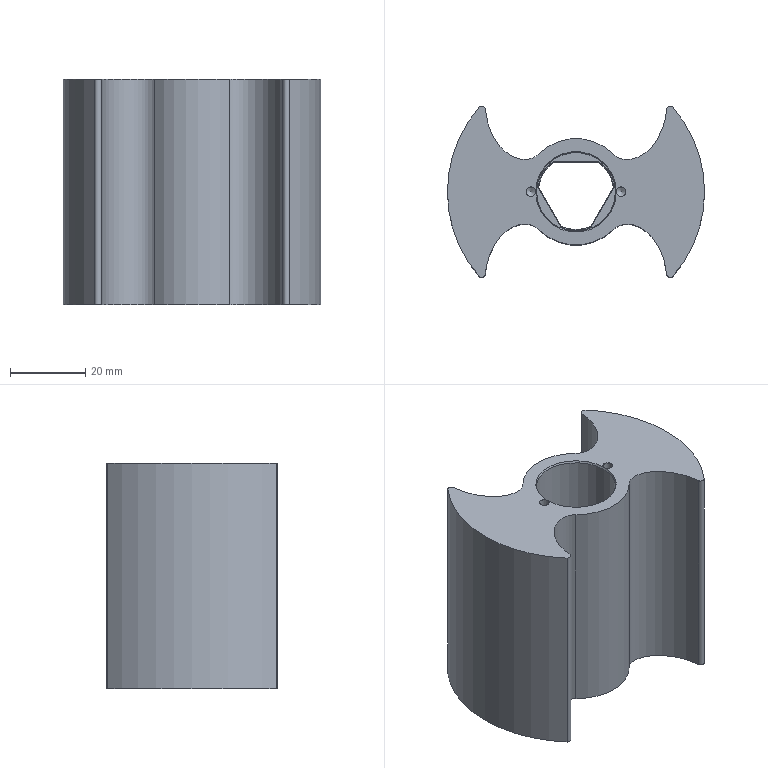Part | 1 solid | 50 faces | box 68.489 x 45.577 x 60 mm | volume 89540 mm3 | cylinder 17 | cone 16 | plane 13 | spline 4 | commonest cylinder face diameters 1.9 x4 20 x3 2.5 x2 4.2 x2 28.311 x2 68.489 x2
STEP:
#1=CARTESIAN_POINT('',(-6.,8.,-50.3));
#2=VERTEX_POINT('',#1);
#3=CARTESIAN_POINT('',(-6.,8.,-15.4));
#4=VERTEX_POINT('',#3);
#5=CARTESIAN_POINT('',(-6.,8.,-60.));
#6=DIRECTION('',(0.,0.,1.));
#7=VECTOR('',#6,1000.);
#8=LINE('',#5,#7);
#9=EDGE_CURVE('',#2,#4,#8,.T.);
#10=ORIENTED_EDGE('',*,*,#9,.T.);
#11=CARTESIAN_POINT('',(-9.928,1.196,-15.4));
#12=VERTEX_POINT('',#11);
#13=CARTESIAN_POINT('',(0.,0.,-15.4));
#14=DIRECTION('',(0.,0.,1.));
#15=DIRECTION('',(1.,0.,0.));
#16=AXIS2_PLACEMENT_3D('',#13,#14,#15);
#17=CIRCLE('',#16,10.);
#18=EDGE_CURVE('',#4,#12,#17,.T.);
#19=ORIENTED_EDGE('',*,*,#18,.T.);
#20=CARTESIAN_POINT('',(-9.928,1.196,-50.3));
#21=VERTEX_POINT('',#20);
#22=CARTESIAN_POINT('',(-9.928,1.196,-60.));
#23=DIRECTION('',(0.,0.,1.));
#24=VECTOR('',#23,1000.);
#25=LINE('',#22,#24);
#26=EDGE_CURVE('',#21,#12,#25,.T.);
#27=ORIENTED_EDGE('',*,*,#26,.F.);
#28=CARTESIAN_POINT('',(0.,0.,-50.3));
#29=DIRECTION('',(0.,0.,-1.));
#30=DIRECTION('',(-1.,0.,0.));
#31=AXIS2_PLACEMENT_3D('',#28,#29,#30);
#32=CIRCLE('',#31,10.);
#33=EDGE_CURVE('',#21,#2,#32,.T.);
#34=ORIENTED_EDGE('',*,*,#33,.T.);
#35=EDGE_LOOP('',(#10,#19,#27,#34));
#36=FACE_BOUND('',#35,.T.);
#37=CARTESIAN_POINT('',(0.,0.,-60.));
#38=DIRECTION('',(0.,0.,1.));
#39=DIRECTION('',(1.,0.,0.));
#40=AXIS2_PLACEMENT_3D('',#37,#38,#39);
#41=CYLINDRICAL_SURFACE('',#40,10.);
#42=ADVANCED_FACE('',(#36),#41,.F.);
#43=CARTESIAN_POINT('',(6.,8.,-50.3));
#44=VERTEX_POINT('',#43);
#45=CARTESIAN_POINT('',(6.,8.,-15.4));
#46=VERTEX_POINT('',#45);
#47=CARTESIAN_POINT('',(6.,8.,-60.));
#48=DIRECTION('',(0.,0.,1.));
#49=VECTOR('',#48,1000.);
#50=LINE('',#47,#49);
#51=EDGE_CURVE('',#44,#46,#50,.T.);
#52=ORIENTED_EDGE('',*,*,#51,.T.);
#53=CARTESIAN_POINT('',(-6.,8.,-15.4));
#54=DIRECTION('',(-1.,0.,0.));
#55=VECTOR('',#54,1000.);
#56=LINE('',#53,#55);
#57=EDGE_CURVE('',#46,#4,#56,.T.);
#58=ORIENTED_EDGE('',*,*,#57,.T.);
#59=ORIENTED_EDGE('',*,*,#9,.F.);
#60=CARTESIAN_POINT('',(6.,8.,-50.3));
#61=DIRECTION('',(1.,0.,0.));
#62=VECTOR('',#61,1000.);
#63=LINE('',#60,#62);
#64=EDGE_CURVE('',#2,#44,#63,.T.);
#65=ORIENTED_EDGE('',*,*,#64,.T.);
#66=EDGE_LOOP('',(#52,#58,#59,#65));
#67=FACE_BOUND('',#66,.T.);
#68=CARTESIAN_POINT('',(-6.,8.,-60.));
#69=DIRECTION('',(0.,1.,0.));
#70=DIRECTION('',(0.,0.,-1.));
#71=AXIS2_PLACEMENT_3D('',#68,#69,#70);
#72=PLANE('',#71);
#73=ADVANCED_FACE('',(#67),#72,.F.);
#74=CARTESIAN_POINT('',(9.928,1.196,-50.3));
#75=VERTEX_POINT('',#74);
#76=CARTESIAN_POINT('',(9.928,1.196,-15.4));
#77=VERTEX_POINT('',#76);
#78=CARTESIAN_POINT('',(9.928,1.196,-60.));
#79=DIRECTION('',(0.,0.,1.));
#80=VECTOR('',#79,1000.);
#81=LINE('',#78,#80);
#82=EDGE_CURVE('',#75,#77,#81,.T.);
#83=ORIENTED_EDGE('',*,*,#82,.T.);
#84=CARTESIAN_POINT('',(0.,0.,-15.4));
#85=DIRECTION('',(0.,0.,1.));
#86=DIRECTION('',(1.,0.,0.));
#87=AXIS2_PLACEMENT_3D('',#84,#85,#86);
#88=CIRCLE('',#87,10.);
#89=EDGE_CURVE('',#77,#46,#88,.T.);
#90=ORIENTED_EDGE('',*,*,#89,.T.);
#91=ORIENTED_EDGE('',*,*,#51,.F.);
#92=CARTESIAN_POINT('',(0.,0.,-50.3));
#93=DIRECTION('',(0.,0.,-1.));
#94=DIRECTION('',(-1.,0.,0.));
#95=AXIS2_PLACEMENT_3D('',#92,#93,#94);
#96=CIRCLE('',#95,10.);
#97=EDGE_CURVE('',#44,#75,#96,.T.);
#98=ORIENTED_EDGE('',*,*,#97,.T.);
#99=EDGE_LOOP('',(#83,#90,#91,#98));
#100=FACE_BOUND('',#99,.T.);
#101=CARTESIAN_POINT('',(0.,0.,-60.));
#102=DIRECTION('',(0.,0.,1.));
#103=DIRECTION('',(1.,0.,0.));
#104=AXIS2_PLACEMENT_3D('',#101,#102,#103);
#105=CYLINDRICAL_SURFACE('',#104,10.);
#106=ADVANCED_FACE('',(#100),#105,.F.);
#107=CARTESIAN_POINT('',(3.928,-9.196,-50.3));
#108=VERTEX_POINT('',#107);
#109=CARTESIAN_POINT('',(3.928,-9.196,-15.4));
#110=VERTEX_POINT('',#109);
#111=CARTESIAN_POINT('',(3.928,-9.196,-60.));
#112=DIRECTION('',(0.,0.,1.));
#113=VECTOR('',#112,1000.);
#114=LINE('',#111,#113);
#115=EDGE_CURVE('',#108,#110,#114,.T.);
#116=ORIENTED_EDGE('',*,*,#115,.T.);
#117=CARTESIAN_POINT('',(9.928,1.196,-15.4));
#118=DIRECTION('',(0.5,0.866,0.));
#119=VECTOR('',#118,1000.);
#120=LINE('',#117,#119);
#121=EDGE_CURVE('',#110,#77,#120,.T.);
#122=ORIENTED_EDGE('',*,*,#121,.T.);
#123=ORIENTED_EDGE('',*,*,#82,.F.);
#124=CARTESIAN_POINT('',(3.928,-9.196,-50.3));
#125=DIRECTION('',(-0.5,-0.866,0.));
#126=VECTOR('',#125,1000.);
#127=LINE('',#124,#126);
#128=EDGE_CURVE('',#75,#108,#127,.T.);
#129=ORIENTED_EDGE('',*,*,#128,.T.);
#130=EDGE_LOOP('',(#116,#122,#123,#129));
#131=FACE_BOUND('',#130,.T.);
#132=CARTESIAN_POINT('',(9.928,1.196,-60.));
#133=DIRECTION('',(0.866,-0.5,0.));
#134=DIRECTION('',(-0.5,-0.866,0.));
#135=AXIS2_PLACEMENT_3D('',#132,#133,#134);
#136=PLANE('',#135);
#137=ADVANCED_FACE('',(#131),#136,.F.);
#138=CARTESIAN_POINT('',(-3.928,-9.196,-50.3));
#139=VERTEX_POINT('',#138);
#140=CARTESIAN_POINT('',(-3.928,-9.196,-15.4));
#141=VERTEX_POINT('',#140);
#142=CARTESIAN_POINT('',(-3.928,-9.196,-60.));
#143=DIRECTION('',(0.,0.,1.));
#144=VECTOR('',#143,1000.);
#145=LINE('',#142,#144);
#146=EDGE_CURVE('',#139,#141,#145,.T.);
#147=ORIENTED_EDGE('',*,*,#146,.T.);
#148=CARTESIAN_POINT('',(0.,0.,-15.4));
#149=DIRECTION('',(0.,0.,1.));
#150=DIRECTION('',(1.,0.,0.));
#151=AXIS2_PLACEMENT_3D('',#148,#149,#150);
#152=CIRCLE('',#151,10.);
#153=EDGE_CURVE('',#141,#110,#152,.T.);
#154=ORIENTED_EDGE('',*,*,#153,.T.);
#155=ORIENTED_EDGE('',*,*,#115,.F.);
#156=CARTESIAN_POINT('',(0.,0.,-50.3));
#157=DIRECTION('',(0.,0.,-1.));
#158=DIRECTION('',(-1.,0.,0.));
#159=AXIS2_PLACEMENT_3D('',#156,#157,#158);
#160=CIRCLE('',#159,10.);
#161=EDGE_CURVE('',#108,#139,#160,.T.);
#162=ORIENTED_EDGE('',*,*,#161,.T.);
#163=EDGE_LOOP('',(#147,#154,#155,#162));
#164=FACE_BOUND('',#163,.T.);
#165=CARTESIAN_POINT('',(0.,0.,-60.));
#166=DIRECTION('',(0.,0.,1.));
#167=DIRECTION('',(1.,0.,0.));
#168=AXIS2_PLACEMENT_3D('',#165,#166,#167);
#169=CYLINDRICAL_SURFACE('',#168,10.);
#170=ADVANCED_FACE('',(#164),#169,.F.);
#171=ORIENTED_EDGE('',*,*,#26,.T.);
#172=CARTESIAN_POINT('',(-3.928,-9.196,-15.4));
#173=DIRECTION('',(0.5,-0.866,0.));
#174=VECTOR('',#173,1000.);
#175=LINE('',#172,#174);
#176=EDGE_CURVE('',#12,#141,#175,.T.);
#177=ORIENTED_EDGE('',*,*,#176,.T.);
#178=ORIENTED_EDGE('',*,*,#146,.F.);
#179=CARTESIAN_POINT('',(-9.928,1.196,-50.3));
#180=DIRECTION('',(-0.5,0.866,0.));
#181=VECTOR('',#180,1000.);
#182=LINE('',#179,#181);
#183=EDGE_CURVE('',#139,#21,#182,.T.);
#184=ORIENTED_EDGE('',*,*,#183,.T.);
#185=EDGE_LOOP('',(#171,#177,#178,#184));
#186=FACE_BOUND('',#185,.T.);
#187=CARTESIAN_POINT('',(-3.928,-9.196,-60.));
#188=DIRECTION('',(-0.866,-0.5,0.));
#189=DIRECTION('',(-0.5,0.866,0.));
#190=AXIS2_PLACEMENT_3D('',#187,#188,#189);
#191=PLANE('',#190);
#192=ADVANCED_FACE('',(#186),#191,.F.);
#193=CARTESIAN_POINT('',(25.849,22.462,0.));
#194=VERTEX_POINT('',#193);
#195=CARTESIAN_POINT('',(25.849,-22.462,0.));
#196=VERTEX_POINT('',#195);
#197=CARTESIAN_POINT('',(0.,0.,0.));
#198=DIRECTION('',(0.,0.,-1.));
#199=DIRECTION('',(-1.,0.,0.));
#200=AXIS2_PLACEMENT_3D('',#197,#198,#199);
#201=CIRCLE('',#200,34.245);
#202=EDGE_CURVE('',#194,#196,#201,.T.);
#203=ORIENTED_EDGE('',*,*,#202,.T.);
#204=CARTESIAN_POINT('',(25.849,-22.462,-60.));
#205=VERTEX_POINT('',#204);
#206=CARTESIAN_POINT('',(25.849,-22.462,-60.));
#207=DIRECTION('',(0.,0.,1.));
#208=VECTOR('',#207,1000.);
#209=LINE('',#206,#208);
#210=EDGE_CURVE('',#205,#196,#209,.T.);
#211=ORIENTED_EDGE('',*,*,#210,.F.);
#212=CARTESIAN_POINT('',(25.849,22.462,-60.));
#213=VERTEX_POINT('',#212);
#214=CARTESIAN_POINT('',(0.,0.,-60.));
#215=DIRECTION('',(0.,0.,-1.));
#216=DIRECTION('',(-1.,0.,0.));
#217=AXIS2_PLACEMENT_3D('',#214,#215,#216);
#218=CIRCLE('',#217,34.245);
#219=EDGE_CURVE('',#213,#205,#218,.T.);
#220=ORIENTED_EDGE('',*,*,#219,.F.);
#221=CARTESIAN_POINT('',(25.849,22.462,-60.));
#222=DIRECTION('',(0.,0.,1.));
#223=VECTOR('',#222,1000.);
#224=LINE('',#221,#223);
#225=EDGE_CURVE('',#213,#194,#224,.T.);
#226=ORIENTED_EDGE('',*,*,#225,.T.);
#227=EDGE_LOOP('',(#203,#211,#220,#226));
#228=FACE_BOUND('',#227,.T.);
#229=CARTESIAN_POINT('',(0.,0.,-60.));
#230=DIRECTION('',(0.,0.,1.));
#231=DIRECTION('',(1.,0.,0.));
#232=AXIS2_PLACEMENT_3D('',#229,#230,#231);
#233=CYLINDRICAL_SURFACE('',#232,34.245);
#234=ADVANCED_FACE('',(#228),#233,.T.);
#235=CARTESIAN_POINT('',(24.186,-21.933,0.));
#236=VERTEX_POINT('',#235);
#237=CARTESIAN_POINT('',(25.132,-21.839,0.));
#238=DIRECTION('',(0.,0.,-1.));
#239=DIRECTION('',(-1.,0.,0.));
#240=AXIS2_PLACEMENT_3D('',#237,#238,#239);
#241=CIRCLE('',#240,0.95);
#242=EDGE_CURVE('',#196,#236,#241,.T.);
#243=ORIENTED_EDGE('',*,*,#242,.T.);
#244=CARTESIAN_POINT('',(24.186,-21.933,-60.));
#245=VERTEX_POINT('',#244);
#246=CARTESIAN_POINT('',(24.186,-21.933,-60.));
#247=DIRECTION('',(0.,0.,1.));
#248=VECTOR('',#247,1000.);
#249=LINE('',#246,#248);
#250=EDGE_CURVE('',#245,#236,#249,.T.);
#251=ORIENTED_EDGE('',*,*,#250,.F.);
#252=CARTESIAN_POINT('',(25.132,-21.839,-60.));
#253=DIRECTION('',(0.,0.,-1.));
#254=DIRECTION('',(-1.,0.,0.));
#255=AXIS2_PLACEMENT_3D('',#252,#253,#254);
#256=CIRCLE('',#255,0.95);
#257=EDGE_CURVE('',#205,#245,#256,.T.);
#258=ORIENTED_EDGE('',*,*,#257,.F.);
#259=ORIENTED_EDGE('',*,*,#210,.T.);
#260=EDGE_LOOP('',(#243,#251,#258,#259));
#261=FACE_BOUND('',#260,.T.);
#262=CARTESIAN_POINT('',(25.132,-21.839,-60.));
#263=DIRECTION('',(0.,0.,1.));
#264=DIRECTION('',(1.,0.,0.));
#265=AXIS2_PLACEMENT_3D('',#262,#263,#264);
#266=CYLINDRICAL_SURFACE('',#265,0.95);
#267=ADVANCED_FACE('',(#261),#266,.T.);
#268=CARTESIAN_POINT('',(10.009,-10.009,0.));
#269=VERTEX_POINT('',#268);
#270=CARTESIAN_POINT('',(24.186,-21.933,0.));
#271=CARTESIAN_POINT('',(23.996,-20.063,0.));
#272=CARTESIAN_POINT('',(23.182,-16.428,0.));
#273=CARTESIAN_POINT('',(20.767,-12.303,0.));
#274=CARTESIAN_POINT('',(17.917,-9.833,0.));
#275=CARTESIAN_POINT('',(15.332,-8.627,0.));
#276=CARTESIAN_POINT('',(12.427,-8.456,0.));
#277=CARTESIAN_POINT('',(10.685,-9.338,0.));
#278=CARTESIAN_POINT('',(10.009,-10.009,0.));
#279=B_SPLINE_CURVE_WITH_KNOTS('',3,(#270,#271,#272,#273,#274,#275,#276,#277,#278),.UNSPECIFIED.,.F.,.F.,(4,1,1,1,1,1,4),(0.,0.005569,0.01114,0.01392,0.01671,0.01949,0.02228),.UNSPECIFIED.);
#280=EDGE_CURVE('',#236,#269,#279,.T.);
#281=ORIENTED_EDGE('',*,*,#280,.T.);
#282=CARTESIAN_POINT('',(10.009,-10.009,-60.));
#283=VERTEX_POINT('',#282);
#284=CARTESIAN_POINT('',(10.009,-10.009,-60.));
#285=DIRECTION('',(0.,0.,1.));
#286=VECTOR('',#285,1000.);
#287=LINE('',#284,#286);
#288=EDGE_CURVE('',#283,#269,#287,.T.);
#289=ORIENTED_EDGE('',*,*,#288,.F.);
#290=CARTESIAN_POINT('',(24.186,-21.933,-60.));
#291=CARTESIAN_POINT('',(23.996,-20.063,-60.));
#292=CARTESIAN_POINT('',(23.182,-16.428,-60.));
#293=CARTESIAN_POINT('',(20.767,-12.303,-60.));
#294=CARTESIAN_POINT('',(17.917,-9.833,-60.));
#295=CARTESIAN_POINT('',(15.332,-8.627,-60.));
#296=CARTESIAN_POINT('',(12.427,-8.456,-60.));
#297=CARTESIAN_POINT('',(10.685,-9.338,-60.));
#298=CARTESIAN_POINT('',(10.009,-10.009,-60.));
#299=B_SPLINE_CURVE_WITH_KNOTS('',3,(#290,#291,#292,#293,#294,#295,#296,#297,#298),.UNSPECIFIED.,.F.,.F.,(4,1,1,1,1,1,4),(0.,0.005569,0.01114,0.01392,0.01671,0.01949,0.02228),.UNSPECIFIED.);
#300=EDGE_CURVE('',#245,#283,#299,.T.);
#301=ORIENTED_EDGE('',*,*,#300,.F.);
#302=ORIENTED_EDGE('',*,*,#250,.T.);
#303=EDGE_LOOP('',(#281,#289,#301,#302));
#304=FACE_BOUND('',#303,.T.);
#305=CARTESIAN_POINT('',(24.186,-21.933,-60.));
#306=CARTESIAN_POINT('',(24.186,-21.933,0.));
#307=CARTESIAN_POINT('',(23.998,-20.077,-60.));
#308=CARTESIAN_POINT('',(23.998,-20.077,0.));
#309=CARTESIAN_POINT('',(23.172,-16.392,-60.));
#310=CARTESIAN_POINT('',(23.172,-16.392,0.));
#311=CARTESIAN_POINT('',(20.758,-12.292,-60.));
#312=CARTESIAN_POINT('',(20.758,-12.292,0.));
#313=CARTESIAN_POINT('',(17.902,-9.822,-60.));
#314=CARTESIAN_POINT('',(17.902,-9.822,0.));
#315=CARTESIAN_POINT('',(15.317,-8.627,-60.));
#316=CARTESIAN_POINT('',(15.317,-8.627,0.));
#317=CARTESIAN_POINT('',(12.431,-8.452,-60.));
#318=CARTESIAN_POINT('',(12.431,-8.452,0.));
#319=CARTESIAN_POINT('',(10.671,-9.352,-60.));
#320=CARTESIAN_POINT('',(10.671,-9.352,0.));
#321=CARTESIAN_POINT('',(10.009,-10.009,-60.));
#322=CARTESIAN_POINT('',(10.009,-10.009,0.));
#323=B_SPLINE_SURFACE_WITH_KNOTS('',3,1,((#305,#306),(#307,#308),(#309,#310),(#311,#312),(#313,#314),(#315,#316),(#317,#318),(#319,#320),(#321,#322)),.SURF_OF_LINEAR_EXTRUSION.,.F.,.F.,.F.,(4,1,1,1,1,1,4),(2,2),(0.,0.25,0.5,0.625,0.75,0.875,1.),(0.,1.),.UNSPECIFIED.);
#324=ADVANCED_FACE('',(#304),#323,.F.);
#325=CARTESIAN_POINT('',(-10.009,-10.009,0.));
#326=VERTEX_POINT('',#325);
#327=CARTESIAN_POINT('',(0.,0.,0.));
#328=DIRECTION('',(0.,0.,-1.));
#329=DIRECTION('',(-1.,0.,0.));
#330=AXIS2_PLACEMENT_3D('',#327,#328,#329);
#331=CIRCLE('',#330,14.155);
#332=EDGE_CURVE('',#269,#326,#331,.T.);
#333=ORIENTED_EDGE('',*,*,#332,.T.);
#334=CARTESIAN_POINT('',(-10.009,-10.009,-60.));
#335=VERTEX_POINT('',#334);
#336=CARTESIAN_POINT('',(-10.009,-10.009,-60.));
#337=DIRECTION('',(0.,0.,1.));
#338=VECTOR('',#337,1000.);
#339=LINE('',#336,#338);
#340=EDGE_CURVE('',#335,#326,#339,.T.);
#341=ORIENTED_EDGE('',*,*,#340,.F.);
#342=CARTESIAN_POINT('',(0.,0.,-60.));
#343=DIRECTION('',(0.,0.,-1.));
#344=DIRECTION('',(-1.,0.,0.));
#345=AXIS2_PLACEMENT_3D('',#342,#343,#344);
#346=CIRCLE('',#345,14.155);
#347=EDGE_CURVE('',#283,#335,#346,.T.);
#348=ORIENTED_EDGE('',*,*,#347,.F.);
#349=ORIENTED_EDGE('',*,*,#288,.T.);
#350=EDGE_LOOP('',(#333,#341,#348,#349));
#351=FACE_BOUND('',#350,.T.);
#352=CARTESIAN_POINT('',(0.,0.,-60.));
#353=DIRECTION('',(0.,0.,1.));
#354=DIRECTION('',(1.,0.,0.));
#355=AXIS2_PLACEMENT_3D('',#352,#353,#354);
#356=CYLINDRICAL_SURFACE('',#355,14.155);
#357=ADVANCED_FACE('',(#351),#356,.T.);
#358=CARTESIAN_POINT('',(-24.186,-21.933,0.));
#359=VERTEX_POINT('',#358);
#360=CARTESIAN_POINT('',(-10.009,-10.009,0.));
#361=CARTESIAN_POINT('',(-10.685,-9.338,0.));
#362=CARTESIAN_POINT('',(-12.423,-8.455,0.));
#363=CARTESIAN_POINT('',(-16.314,-8.693,0.));
#364=CARTESIAN_POINT('',(-20.3,-11.5,0.));
#365=CARTESIAN_POINT('',(-23.18,-16.426,0.));
#366=CARTESIAN_POINT('',(-23.996,-20.064,0.));
#367=CARTESIAN_POINT('',(-24.186,-21.933,0.));
#368=B_SPLINE_CURVE_WITH_KNOTS('',3,(#360,#361,#362,#363,#364,#365,#366,#367),.UNSPECIFIED.,.F.,.F.,(4,1,1,1,1,4),(0.,0.002815,0.00563,0.01126,0.01689,0.02252),.UNSPECIFIED.);
#369=EDGE_CURVE('',#326,#359,#368,.T.);
#370=ORIENTED_EDGE('',*,*,#369,.T.);
#371=CARTESIAN_POINT('',(-24.186,-21.933,-60.));
#372=VERTEX_POINT('',#371);
#373=CARTESIAN_POINT('',(-24.186,-21.933,-60.));
#374=DIRECTION('',(0.,0.,1.));
#375=VECTOR('',#374,1000.);
#376=LINE('',#373,#375);
#377=EDGE_CURVE('',#372,#359,#376,.T.);
#378=ORIENTED_EDGE('',*,*,#377,.F.);
#379=CARTESIAN_POINT('',(-10.009,-10.009,-60.));
#380=CARTESIAN_POINT('',(-10.685,-9.338,-60.));
#381=CARTESIAN_POINT('',(-12.423,-8.455,-60.));
#382=CARTESIAN_POINT('',(-16.314,-8.693,-60.));
#383=CARTESIAN_POINT('',(-20.3,-11.5,-60.));
#384=CARTESIAN_POINT('',(-23.18,-16.426,-60.));
#385=CARTESIAN_POINT('',(-23.996,-20.064,-60.));
#386=CARTESIAN_POINT('',(-24.186,-21.933,-60.));
#387=B_SPLINE_CURVE_WITH_KNOTS('',3,(#379,#380,#381,#382,#383,#384,#385,#386),.UNSPECIFIED.,.F.,.F.,(4,1,1,1,1,4),(0.,0.002815,0.00563,0.01126,0.01689,0.02252),.UNSPECIFIED.);
#388=EDGE_CURVE('',#335,#372,#387,.T.);
#389=ORIENTED_EDGE('',*,*,#388,.F.);
#390=ORIENTED_EDGE('',*,*,#340,.T.);
#391=EDGE_LOOP('',(#370,#378,#389,#390));
#392=FACE_BOUND('',#391,.T.);
#393=CARTESIAN_POINT('',(-10.009,-10.009,-60.));
#394=CARTESIAN_POINT('',(-10.009,-10.009,0.));
#395=CARTESIAN_POINT('',(-10.671,-9.352,-60.));
#396=CARTESIAN_POINT('',(-10.671,-9.352,0.));
#397=CARTESIAN_POINT('',(-12.431,-8.452,-60.));
#398=CARTESIAN_POINT('',(-12.431,-8.452,0.));
#399=CARTESIAN_POINT('',(-15.317,-8.627,-60.));
#400=CARTESIAN_POINT('',(-15.317,-8.627,0.));
#401=CARTESIAN_POINT('',(-17.902,-9.822,-60.));
#402=CARTESIAN_POINT('',(-17.902,-9.822,0.));
#403=CARTESIAN_POINT('',(-20.758,-12.292,-60.));
#404=CARTESIAN_POINT('',(-20.758,-12.292,0.));
#405=CARTESIAN_POINT('',(-23.172,-16.392,-60.));
#406=CARTESIAN_POINT('',(-23.172,-16.392,0.));
#407=CARTESIAN_POINT('',(-23.998,-20.077,-60.));
#408=CARTESIAN_POINT('',(-23.998,-20.077,0.));
#409=CARTESIAN_POINT('',(-24.186,-21.933,-60.));
#410=CARTESIAN_POINT('',(-24.186,-21.933,0.));
#411=B_SPLINE_SURFACE_WITH_KNOTS('',3,1,((#393,#394),(#395,#396),(#397,#398),(#399,#400),(#401,#402),(#403,#404),(#405,#406),(#407,#408),(#409,#410)),.SURF_OF_LINEAR_EXTRUSION.,.F.,.F.,.F.,(4,1,1,1,1,1,4),(2,2),(-0.000003121,0.125,0.25,0.375,0.5,0.75,1.),(0.,1.),.UNSPECIFIED.);
#412=ADVANCED_FACE('',(#392),#411,.F.);
#413=CARTESIAN_POINT('',(-25.849,-22.462,0.));
#414=VERTEX_POINT('',#413);
#415=CARTESIAN_POINT('',(-25.132,-21.839,0.));
#416=DIRECTION('',(0.,0.,-1.));
#417=DIRECTION('',(-1.,0.,0.));
#418=AXIS2_PLACEMENT_3D('',#415,#416,#417);
#419=CIRCLE('',#418,0.95);
#420=EDGE_CURVE('',#359,#414,#419,.T.);
#421=ORIENTED_EDGE('',*,*,#420,.T.);
#422=CARTESIAN_POINT('',(-25.849,-22.462,-60.));
#423=VERTEX_POINT('',#422);
#424=CARTESIAN_POINT('',(-25.849,-22.462,-60.));
#425=DIRECTION('',(0.,0.,1.));
#426=VECTOR('',#425,1000.);
#427=LINE('',#424,#426);
#428=EDGE_CURVE('',#423,#414,#427,.T.);
#429=ORIENTED_EDGE('',*,*,#428,.F.);
#430=CARTESIAN_POINT('',(-25.132,-21.839,-60.));
#431=DIRECTION('',(0.,0.,-1.));
#432=DIRECTION('',(-1.,0.,0.));
#433=AXIS2_PLACEMENT_3D('',#430,#431,#432);
#434=CIRCLE('',#433,0.95);
#435=EDGE_CURVE('',#372,#423,#434,.T.);
#436=ORIENTED_EDGE('',*,*,#435,.F.);
#437=ORIENTED_EDGE('',*,*,#377,.T.);
#438=EDGE_LOOP('',(#421,#429,#436,#437));
#439=FACE_BOUND('',#438,.T.);
#440=CARTESIAN_POINT('',(-25.132,-21.839,-60.));
#441=DIRECTION('',(0.,0.,1.));
#442=DIRECTION('',(1.,0.,0.));
#443=AXIS2_PLACEMENT_3D('',#440,#441,#442);
#444=CYLINDRICAL_SURFACE('',#443,0.95);
#445=ADVANCED_FACE('',(#439),#444,.T.);
#446=CARTESIAN_POINT('',(-25.849,22.462,0.));
#447=VERTEX_POINT('',#446);
#448=CARTESIAN_POINT('',(0.,0.,0.));
#449=DIRECTION('',(0.,0.,-1.));
#450=DIRECTION('',(-1.,0.,0.));
#451=AXIS2_PLACEMENT_3D('',#448,#449,#450);
#452=CIRCLE('',#451,34.245);
#453=EDGE_CURVE('',#414,#447,#452,.T.);
#454=ORIENTED_EDGE('',*,*,#453,.T.);
#455=CARTESIAN_POINT('',(-25.849,22.462,-60.));
#456=VERTEX_POINT('',#455);
#457=CARTESIAN_POINT('',(-25.849,22.462,-60.));
#458=DIRECTION('',(0.,0.,1.));
#459=VECTOR('',#458,1000.);
#460=LINE('',#457,#459);
#461=EDGE_CURVE('',#456,#447,#460,.T.);
#462=ORIENTED_EDGE('',*,*,#461,.F.);
#463=CARTESIAN_POINT('',(0.,0.,-60.));
#464=DIRECTION('',(0.,0.,-1.));
#465=DIRECTION('',(-1.,0.,0.));
#466=AXIS2_PLACEMENT_3D('',#463,#464,#465);
#467=CIRCLE('',#466,34.245);
#468=EDGE_CURVE('',#423,#456,#467,.T.);
#469=ORIENTED_EDGE('',*,*,#468,.F.);
#470=ORIENTED_EDGE('',*,*,#428,.T.);
#471=EDGE_LOOP('',(#454,#462,#469,#470));
#472=FACE_BOUND('',#471,.T.);
#473=CARTESIAN_POINT('',(0.,0.,-60.));
#474=DIRECTION('',(0.,0.,1.));
#475=DIRECTION('',(1.,0.,0.));
#476=AXIS2_PLACEMENT_3D('',#473,#474,#475);
#477=CYLINDRICAL_SURFACE('',#476,34.245);
#478=ADVANCED_FACE('',(#472),#477,.T.);
#479=CARTESIAN_POINT('',(-24.186,21.933,0.));
#480=VERTEX_POINT('',#479);
#481=CARTESIAN_POINT('',(-25.132,21.839,0.));
#482=DIRECTION('',(0.,0.,-1.));
#483=DIRECTION('',(-1.,0.,0.));
#484=AXIS2_PLACEMENT_3D('',#481,#482,#483);
#485=CIRCLE('',#484,0.95);
#486=EDGE_CURVE('',#447,#480,#485,.T.);
#487=ORIENTED_EDGE('',*,*,#486,.T.);
#488=CARTESIAN_POINT('',(-24.186,21.933,-60.));
#489=VERTEX_POINT('',#488);
#490=CARTESIAN_POINT('',(-24.186,21.933,-60.));
#491=DIRECTION('',(0.,0.,1.));
#492=VECTOR('',#491,1000.);
#493=LINE('',#490,#492);
#494=EDGE_CURVE('',#489,#480,#493,.T.);
#495=ORIENTED_EDGE('',*,*,#494,.F.);
#496=CARTESIAN_POINT('',(-25.132,21.839,-60.));
#497=DIRECTION('',(0.,0.,-1.));
#498=DIRECTION('',(-1.,0.,0.));
#499=AXIS2_PLACEMENT_3D('',#496,#497,#498);
#500=CIRCLE('',#499,0.95);
#501=EDGE_CURVE('',#456,#489,#500,.T.);
#502=ORIENTED_EDGE('',*,*,#501,.F.);
#503=ORIENTED_EDGE('',*,*,#461,.T.);
#504=EDGE_LOOP('',(#487,#495,#502,#503));
#505=FACE_BOUND('',#504,.T.);
#506=CARTESIAN_POINT('',(-25.132,21.839,-60.));
#507=DIRECTION('',(0.,0.,1.));
#508=DIRECTION('',(1.,0.,0.));
#509=AXIS2_PLACEMENT_3D('',#506,#507,#508);
#510=CYLINDRICAL_SURFACE('',#509,0.95);
#511=ADVANCED_FACE('',(#505),#510,.T.);
#512=CARTESIAN_POINT('',(-10.009,10.009,0.));
#513=VERTEX_POINT('',#512);
#514=CARTESIAN_POINT('',(-24.186,21.933,0.));
#515=CARTESIAN_POINT('',(-23.996,20.063,0.));
#516=CARTESIAN_POINT('',(-23.182,16.428,0.));
#517=CARTESIAN_POINT('',(-20.767,12.303,0.));
#518=CARTESIAN_POINT('',(-17.917,9.833,0.));
#519=CARTESIAN_POINT('',(-15.332,8.627,0.));
#520=CARTESIAN_POINT('',(-12.427,8.456,0.));
#521=CARTESIAN_POINT('',(-10.685,9.338,0.));
#522=CARTESIAN_POINT('',(-10.009,10.009,0.));
#523=B_SPLINE_CURVE_WITH_KNOTS('',3,(#514,#515,#516,#517,#518,#519,#520,#521,#522),.UNSPECIFIED.,.F.,.F.,(4,1,1,1,1,1,4),(0.,0.005569,0.01114,0.01392,0.01671,0.01949,0.02228),.UNSPECIFIED.);
#524=EDGE_CURVE('',#480,#513,#523,.T.);
#525=ORIENTED_EDGE('',*,*,#524,.T.);
#526=CARTESIAN_POINT('',(-10.009,10.009,-60.));
#527=VERTEX_POINT('',#526);
#528=CARTESIAN_POINT('',(-10.009,10.009,-60.));
#529=DIRECTION('',(0.,0.,1.));
#530=VECTOR('',#529,1000.);
#531=LINE('',#528,#530);
#532=EDGE_CURVE('',#527,#513,#531,.T.);
#533=ORIENTED_EDGE('',*,*,#532,.F.);
#534=CARTESIAN_POINT('',(-24.186,21.933,-60.));
#535=CARTESIAN_POINT('',(-23.996,20.063,-60.));
#536=CARTESIAN_POINT('',(-23.182,16.428,-60.));
#537=CARTESIAN_POINT('',(-20.767,12.303,-60.));
#538=CARTESIAN_POINT('',(-17.917,9.833,-60.));
#539=CARTESIAN_POINT('',(-15.332,8.627,-60.));
#540=CARTESIAN_POINT('',(-12.427,8.456,-60.));
#541=CARTESIAN_POINT('',(-10.685,9.338,-60.));
#542=CARTESIAN_POINT('',(-10.009,10.009,-60.));
#543=B_SPLINE_CURVE_WITH_KNOTS('',3,(#534,#535,#536,#537,#538,#539,#540,#541,#542),.UNSPECIFIED.,.F.,.F.,(4,1,1,1,1,1,4),(0.,0.005569,0.01114,0.01392,0.01671,0.01949,0.02228),.UNSPECIFIED.);
#544=EDGE_CURVE('',#489,#527,#543,.T.);
#545=ORIENTED_EDGE('',*,*,#544,.F.);
#546=ORIENTED_EDGE('',*,*,#494,.T.);
#547=EDGE_LOOP('',(#525,#533,#545,#546));
#548=FACE_BOUND('',#547,.T.);
#549=CARTESIAN_POINT('',(-24.186,21.933,-60.));
#550=CARTESIAN_POINT('',(-24.186,21.933,0.));
#551=CARTESIAN_POINT('',(-23.998,20.077,-60.));
#552=CARTESIAN_POINT('',(-23.998,20.077,0.));
#553=CARTESIAN_POINT('',(-23.172,16.392,-60.));
#554=CARTESIAN_POINT('',(-23.172,16.392,0.));
#555=CARTESIAN_POINT('',(-20.758,12.292,-60.));
#556=CARTESIAN_POINT('',(-20.758,12.292,0.));
#557=CARTESIAN_POINT('',(-17.902,9.822,-60.));
#558=CARTESIAN_POINT('',(-17.902,9.822,0.));
#559=CARTESIAN_POINT('',(-15.317,8.627,-60.));
#560=CARTESIAN_POINT('',(-15.317,8.627,0.));
#561=CARTESIAN_POINT('',(-12.431,8.452,-60.));
#562=CARTESIAN_POINT('',(-12.431,8.452,0.));
#563=CARTESIAN_POINT('',(-10.671,9.352,-60.));
#564=CARTESIAN_POINT('',(-10.671,9.352,0.));
#565=CARTESIAN_POINT('',(-10.009,10.009,-60.));
#566=CARTESIAN_POINT('',(-10.009,10.009,0.));
#567=B_SPLINE_SURFACE_WITH_KNOTS('',3,1,((#549,#550),(#551,#552),(#553,#554),(#555,#556),(#557,#558),(#559,#560),(#561,#562),(#563,#564),(#565,#566)),.SURF_OF_LINEAR_EXTRUSION.,.F.,.F.,.F.,(4,1,1,1,1,1,4),(2,2),(0.,0.25,0.5,0.625,0.75,0.875,1.),(0.,1.),.UNSPECIFIED.);
#568=ADVANCED_FACE('',(#548),#567,.F.);
#569=CARTESIAN_POINT('',(10.009,10.009,0.));
#570=VERTEX_POINT('',#569);
#571=CARTESIAN_POINT('',(0.,0.,0.));
#572=DIRECTION('',(0.,0.,-1.));
#573=DIRECTION('',(-1.,0.,0.));
#574=AXIS2_PLACEMENT_3D('',#571,#572,#573);
#575=CIRCLE('',#574,14.155);
#576=EDGE_CURVE('',#513,#570,#575,.T.);
#577=ORIENTED_EDGE('',*,*,#576,.T.);
#578=CARTESIAN_POINT('',(10.009,10.009,-60.));
#579=VERTEX_POINT('',#578);
#580=CARTESIAN_POINT('',(10.009,10.009,-60.));
#581=DIRECTION('',(0.,0.,1.));
#582=VECTOR('',#581,1000.);
#583=LINE('',#580,#582);
#584=EDGE_CURVE('',#579,#570,#583,.T.);
#585=ORIENTED_EDGE('',*,*,#584,.F.);
#586=CARTESIAN_POINT('',(0.,0.,-60.));
#587=DIRECTION('',(0.,0.,-1.));
#588=DIRECTION('',(-1.,0.,0.));
#589=AXIS2_PLACEMENT_3D('',#586,#587,#588);
#590=CIRCLE('',#589,14.155);
#591=EDGE_CURVE('',#527,#579,#590,.T.);
#592=ORIENTED_EDGE('',*,*,#591,.F.);
#593=ORIENTED_EDGE('',*,*,#532,.T.);
#594=EDGE_LOOP('',(#577,#585,#592,#593));
#595=FACE_BOUND('',#594,.T.);
#596=CARTESIAN_POINT('',(0.,0.,-60.));
#597=DIRECTION('',(0.,0.,1.));
#598=DIRECTION('',(1.,0.,0.));
#599=AXIS2_PLACEMENT_3D('',#596,#597,#598);
#600=CYLINDRICAL_SURFACE('',#599,14.155);
#601=ADVANCED_FACE('',(#595),#600,.T.);
#602=CARTESIAN_POINT('',(24.186,21.933,0.));
#603=VERTEX_POINT('',#602);
#604=CARTESIAN_POINT('',(10.009,10.009,0.));
#605=CARTESIAN_POINT('',(10.685,9.338,0.));
#606=CARTESIAN_POINT('',(12.423,8.455,0.));
#607=CARTESIAN_POINT('',(16.314,8.693,0.));
#608=CARTESIAN_POINT('',(20.3,11.5,0.));
#609=CARTESIAN_POINT('',(23.18,16.426,0.));
#610=CARTESIAN_POINT('',(23.996,20.064,0.));
#611=CARTESIAN_POINT('',(24.186,21.933,0.));
#612=B_SPLINE_CURVE_WITH_KNOTS('',3,(#604,#605,#606,#607,#608,#609,#610,#611),.UNSPECIFIED.,.F.,.F.,(4,1,1,1,1,4),(0.,0.002815,0.00563,0.01126,0.01689,0.02252),.UNSPECIFIED.);
#613=EDGE_CURVE('',#570,#603,#612,.T.);
#614=ORIENTED_EDGE('',*,*,#613,.T.);
#615=CARTESIAN_POINT('',(24.186,21.933,-60.));
#616=VERTEX_POINT('',#615);
#617=CARTESIAN_POINT('',(24.186,21.933,-60.));
#618=DIRECTION('',(0.,0.,1.));
#619=VECTOR('',#618,1000.);
#620=LINE('',#617,#619);
#621=EDGE_CURVE('',#616,#603,#620,.T.);
#622=ORIENTED_EDGE('',*,*,#621,.F.);
#623=CARTESIAN_POINT('',(10.009,10.009,-60.));
#624=CARTESIAN_POINT('',(10.685,9.338,-60.));
#625=CARTESIAN_POINT('',(12.423,8.455,-60.));
#626=CARTESIAN_POINT('',(16.314,8.693,-60.));
#627=CARTESIAN_POINT('',(20.3,11.5,-60.));
#628=CARTESIAN_POINT('',(23.18,16.426,-60.));
#629=CARTESIAN_POINT('',(23.996,20.064,-60.));
#630=CARTESIAN_POINT('',(24.186,21.933,-60.));
#631=B_SPLINE_CURVE_WITH_KNOTS('',3,(#623,#624,#625,#626,#627,#628,#629,#630),.UNSPECIFIED.,.F.,.F.,(4,1,1,1,1,4),(0.,0.002815,0.00563,0.01126,0.01689,0.02252),.UNSPECIFIED.);
#632=EDGE_CURVE('',#579,#616,#631,.T.);
#633=ORIENTED_EDGE('',*,*,#632,.F.);
#634=ORIENTED_EDGE('',*,*,#584,.T.);
#635=EDGE_LOOP('',(#614,#622,#633,#634));
#636=FACE_BOUND('',#635,.T.);
#637=CARTESIAN_POINT('',(10.009,10.009,-60.));
#638=CARTESIAN_POINT('',(10.009,10.009,0.));
#639=CARTESIAN_POINT('',(10.671,9.352,-60.));
#640=CARTESIAN_POINT('',(10.671,9.352,0.));
#641=CARTESIAN_POINT('',(12.431,8.452,-60.));
#642=CARTESIAN_POINT('',(12.431,8.452,0.));
#643=CARTESIAN_POINT('',(15.317,8.627,-60.));
#644=CARTESIAN_POINT('',(15.317,8.627,0.));
#645=CARTESIAN_POINT('',(17.902,9.822,-60.));
#646=CARTESIAN_POINT('',(17.902,9.822,0.));
#647=CARTESIAN_POINT('',(20.758,12.292,-60.));
#648=CARTESIAN_POINT('',(20.758,12.292,0.));
#649=CARTESIAN_POINT('',(23.172,16.392,-60.));
#650=CARTESIAN_POINT('',(23.172,16.392,0.));
#651=CARTESIAN_POINT('',(23.998,20.077,-60.));
#652=CARTESIAN_POINT('',(23.998,20.077,0.));
#653=CARTESIAN_POINT('',(24.186,21.933,-60.));
#654=CARTESIAN_POINT('',(24.186,21.933,0.));
#655=B_SPLINE_SURFACE_WITH_KNOTS('',3,1,((#637,#638),(#639,#640),(#641,#642),(#643,#644),(#645,#646),(#647,#648),(#649,#650),(#651,#652),(#653,#654)),.SURF_OF_LINEAR_EXTRUSION.,.F.,.F.,.F.,(4,1,1,1,1,1,4),(2,2),(-0.000003121,0.125,0.25,0.375,0.5,0.75,1.),(0.,1.),.UNSPECIFIED.);
#656=ADVANCED_FACE('',(#636),#655,.F.);
#657=CARTESIAN_POINT('',(25.132,21.839,0.));
#658=DIRECTION('',(0.,0.,-1.));
#659=DIRECTION('',(-1.,0.,0.));
#660=AXIS2_PLACEMENT_3D('',#657,#658,#659);
#661=CIRCLE('',#660,0.95);
#662=EDGE_CURVE('',#603,#194,#661,.T.);
#663=ORIENTED_EDGE('',*,*,#662,.T.);
#664=ORIENTED_EDGE('',*,*,#225,.F.);
#665=CARTESIAN_POINT('',(25.132,21.839,-60.));
#666=DIRECTION('',(0.,0.,-1.));
#667=DIRECTION('',(-1.,0.,0.));
#668=AXIS2_PLACEMENT_3D('',#665,#666,#667);
#669=CIRCLE('',#668,0.95);
#670=EDGE_CURVE('',#616,#213,#669,.T.);
#671=ORIENTED_EDGE('',*,*,#670,.F.);
#672=ORIENTED_EDGE('',*,*,#621,.T.);
#673=EDGE_LOOP('',(#663,#664,#671,#672));
#674=FACE_BOUND('',#673,.T.);
#675=CARTESIAN_POINT('',(25.132,21.839,-60.));
#676=DIRECTION('',(0.,0.,1.));
#677=DIRECTION('',(1.,0.,0.));
#678=AXIS2_PLACEMENT_3D('',#675,#676,#677);
#679=CYLINDRICAL_SURFACE('',#678,0.95);
#680=ADVANCED_FACE('',(#674),#679,.T.);
#681=CARTESIAN_POINT('',(17.25,0.,-60.));
#682=VERTEX_POINT('',#681);
#683=CARTESIAN_POINT('',(20.,0.,-60.));
#684=DIRECTION('',(0.,0.,-1.));
#685=DIRECTION('',(-1.,0.,0.));
#686=AXIS2_PLACEMENT_3D('',#683,#684,#685);
#687=CIRCLE('',#686,2.75);
#688=EDGE_CURVE('',#682,#682,#687,.T.);
#689=ORIENTED_EDGE('',*,*,#688,.F.);
#690=EDGE_LOOP('',(#689));
#691=FACE_BOUND('',#690,.T.);
#692=CARTESIAN_POINT('',(-22.75,0.,-60.));
#693=VERTEX_POINT('',#692);
#694=CARTESIAN_POINT('',(-20.,0.,-60.));
#695=DIRECTION('',(0.,0.,-1.));
#696=DIRECTION('',(-1.,0.,0.));
#697=AXIS2_PLACEMENT_3D('',#694,#695,#696);
#698=CIRCLE('',#697,2.75);
#699=EDGE_CURVE('',#693,#693,#698,.T.);
#700=ORIENTED_EDGE('',*,*,#699,.F.);
#701=EDGE_LOOP('',(#700));
#702=FACE_BOUND('',#701,.T.);
#703=CARTESIAN_POINT('',(-12.2,0.,-60.));
#704=VERTEX_POINT('',#703);
#705=CARTESIAN_POINT('',(0.,0.,-60.));
#706=DIRECTION('',(0.,0.,-1.));
#707=DIRECTION('',(-1.,0.,0.));
#708=AXIS2_PLACEMENT_3D('',#705,#706,#707);
#709=CIRCLE('',#708,12.2);
#710=EDGE_CURVE('',#704,#704,#709,.F.);
#711=ORIENTED_EDGE('',*,*,#710,.T.);
#712=EDGE_LOOP('',(#711));
#713=FACE_BOUND('',#712,.T.);
#714=ORIENTED_EDGE('',*,*,#219,.T.);
#715=ORIENTED_EDGE('',*,*,#257,.T.);
#716=ORIENTED_EDGE('',*,*,#300,.T.);
#717=ORIENTED_EDGE('',*,*,#347,.T.);
#718=ORIENTED_EDGE('',*,*,#388,.T.);
#719=ORIENTED_EDGE('',*,*,#435,.T.);
#720=ORIENTED_EDGE('',*,*,#468,.T.);
#721=ORIENTED_EDGE('',*,*,#501,.T.);
#722=ORIENTED_EDGE('',*,*,#544,.T.);
#723=ORIENTED_EDGE('',*,*,#591,.T.);
#724=ORIENTED_EDGE('',*,*,#632,.T.);
#725=ORIENTED_EDGE('',*,*,#670,.T.);
#726=EDGE_LOOP('',(#714,#715,#716,#717,#718,#719,#720,#721,#722,#723,#724,#725));
#727=FACE_BOUND('',#726,.T.);
#728=CARTESIAN_POINT('',(0.,0.,-60.));
#729=DIRECTION('',(0.,0.,-1.));
#730=DIRECTION('',(-1.,0.,0.));
#731=AXIS2_PLACEMENT_3D('',#728,#729,#730);
#732=PLANE('',#731);
#733=ADVANCED_FACE('',(#691,#702,#713,#727),#732,.T.);
#734=CARTESIAN_POINT('',(10.73,-0.2759,0.));
#735=VERTEX_POINT('',#734);
#736=CARTESIAN_POINT('',(-10.73,-0.2759,0.));
#737=VERTEX_POINT('',#736);
#738=CARTESIAN_POINT('',(0.,0.,0.));
#739=DIRECTION('',(0.,0.,-1.));
#740=DIRECTION('',(-1.,0.,0.));
#741=AXIS2_PLACEMENT_3D('',#738,#739,#740);
#742=CIRCLE('',#741,10.733);
#743=EDGE_CURVE('',#735,#737,#742,.T.);
#744=ORIENTED_EDGE('',*,*,#743,.T.);
#745=CARTESIAN_POINT('',(-10.73,0.2759,0.));
#746=VERTEX_POINT('',#745);
#747=CARTESIAN_POINT('',(-12.,0.,0.));
#748=DIRECTION('',(0.,0.,1.));
#749=DIRECTION('',(1.,0.,0.));
#750=AXIS2_PLACEMENT_3D('',#747,#748,#749);
#751=CIRCLE('',#750,1.3);
#752=EDGE_CURVE('',#746,#737,#751,.T.);
#753=ORIENTED_EDGE('',*,*,#752,.F.);
#754=CARTESIAN_POINT('',(10.73,0.2759,0.));
#755=VERTEX_POINT('',#754);
#756=CARTESIAN_POINT('',(0.,0.,0.));
#757=DIRECTION('',(0.,0.,-1.));
#758=DIRECTION('',(-1.,0.,0.));
#759=AXIS2_PLACEMENT_3D('',#756,#757,#758);
#760=CIRCLE('',#759,10.733);
#761=EDGE_CURVE('',#746,#755,#760,.T.);
#762=ORIENTED_EDGE('',*,*,#761,.T.);
#763=CARTESIAN_POINT('',(12.,0.,0.));
#764=DIRECTION('',(0.,0.,1.));
#765=DIRECTION('',(1.,0.,0.));
#766=AXIS2_PLACEMENT_3D('',#763,#764,#765);
#767=CIRCLE('',#766,1.3);
#768=EDGE_CURVE('',#735,#755,#767,.T.);
#769=ORIENTED_EDGE('',*,*,#768,.F.);
#770=EDGE_LOOP('',(#744,#753,#762,#769));
#771=FACE_BOUND('',#770,.T.);
#772=ORIENTED_EDGE('',*,*,#202,.F.);
#773=ORIENTED_EDGE('',*,*,#662,.F.);
#774=ORIENTED_EDGE('',*,*,#613,.F.);
#775=ORIENTED_EDGE('',*,*,#576,.F.);
#776=ORIENTED_EDGE('',*,*,#524,.F.);
#777=ORIENTED_EDGE('',*,*,#486,.F.);
#778=ORIENTED_EDGE('',*,*,#453,.F.);
#779=ORIENTED_EDGE('',*,*,#420,.F.);
#780=ORIENTED_EDGE('',*,*,#369,.F.);
#781=ORIENTED_EDGE('',*,*,#332,.F.);
#782=ORIENTED_EDGE('',*,*,#280,.F.);
#783=ORIENTED_EDGE('',*,*,#242,.F.);
#784=EDGE_LOOP('',(#772,#773,#774,#775,#776,#777,#778,#779,#780,#781,#782,#783));
#785=FACE_BOUND('',#784,.T.);
#786=CARTESIAN_POINT('',(0.,0.,0.));
#787=DIRECTION('',(0.,0.,-1.));
#788=DIRECTION('',(-1.,0.,0.));
#789=AXIS2_PLACEMENT_3D('',#786,#787,#788);
#790=PLANE('',#789);
#791=ADVANCED_FACE('',(#771,#785),#790,.F.);
#792=CARTESIAN_POINT('',(-10.5,0.,-0.5));
#793=VERTEX_POINT('',#792);
#794=CARTESIAN_POINT('',(0.,0.,-0.5));
#795=DIRECTION('',(0.,0.,-1.));
#796=DIRECTION('',(-1.,0.,0.));
#797=AXIS2_PLACEMENT_3D('',#794,#795,#796);
#798=CIRCLE('',#797,10.5);
#799=EDGE_CURVE('',#793,#793,#798,.F.);
#800=ORIENTED_EDGE('',*,*,#799,.T.);
#801=EDGE_LOOP('',(#800));
#802=FACE_BOUND('',#801,.T.);
#803=CARTESIAN_POINT('',(10.5,0.,-15.2));
#804=VERTEX_POINT('',#803);
#805=CARTESIAN_POINT('',(0.,0.,-15.2));
#806=DIRECTION('',(0.,0.,1.));
#807=DIRECTION('',(1.,0.,0.));
#808=AXIS2_PLACEMENT_3D('',#805,#806,#807);
#809=CIRCLE('',#808,10.5);
#810=EDGE_CURVE('',#804,#804,#809,.T.);
#811=ORIENTED_EDGE('',*,*,#810,.F.);
#812=EDGE_LOOP('',(#811));
#813=FACE_BOUND('',#812,.T.);
#814=CARTESIAN_POINT('',(0.,0.,-15.2));
#815=DIRECTION('',(0.,0.,1.));
#816=DIRECTION('',(1.,0.,0.));
#817=AXIS2_PLACEMENT_3D('',#814,#815,#816);
#818=CYLINDRICAL_SURFACE('',#817,10.5);
#819=ADVANCED_FACE('',(#802,#813),#818,.F.);
#820=CARTESIAN_POINT('',(10.135,1.154,-15.2));
#821=VERTEX_POINT('',#820);
#822=CARTESIAN_POINT('',(4.068,-9.354,-15.2));
#823=VERTEX_POINT('',#822);
#824=CARTESIAN_POINT('',(4.101,-9.296,-15.2));
#825=DIRECTION('',(-0.5,-0.866,0.));
#826=VECTOR('',#825,1000.);
#827=LINE('',#824,#826);
#828=EDGE_CURVE('',#821,#823,#827,.T.);
#829=ORIENTED_EDGE('',*,*,#828,.T.);
#830=CARTESIAN_POINT('',(-4.068,-9.354,-15.2));
#831=VERTEX_POINT('',#830);
#832=CARTESIAN_POINT('',(0.,0.,-15.2));
#833=DIRECTION('',(0.,0.,1.));
#834=DIRECTION('',(1.,0.,0.));
#835=AXIS2_PLACEMENT_3D('',#832,#833,#834);
#836=CIRCLE('',#835,10.2);
#837=EDGE_CURVE('',#823,#831,#836,.F.);
#838=ORIENTED_EDGE('',*,*,#837,.T.);
#839=CARTESIAN_POINT('',(-10.135,1.154,-15.2));
#840=VERTEX_POINT('',#839);
#841=CARTESIAN_POINT('',(-10.101,1.096,-15.2));
#842=DIRECTION('',(-0.5,0.866,0.));
#843=VECTOR('',#842,1000.);
#844=LINE('',#841,#843);
#845=EDGE_CURVE('',#831,#840,#844,.T.);
#846=ORIENTED_EDGE('',*,*,#845,.T.);
#847=CARTESIAN_POINT('',(-6.066,8.2,-15.2));
#848=VERTEX_POINT('',#847);
#849=CARTESIAN_POINT('',(0.,0.,-15.2));
#850=DIRECTION('',(0.,0.,1.));
#851=DIRECTION('',(1.,0.,0.));
#852=AXIS2_PLACEMENT_3D('',#849,#850,#851);
#853=CIRCLE('',#852,10.2);
#854=EDGE_CURVE('',#840,#848,#853,.F.);
#855=ORIENTED_EDGE('',*,*,#854,.T.);
#856=CARTESIAN_POINT('',(6.066,8.2,-15.2));
#857=VERTEX_POINT('',#856);
#858=CARTESIAN_POINT('',(6.,8.2,-15.2));
#859=DIRECTION('',(1.,0.,0.));
#860=VECTOR('',#859,1000.);
#861=LINE('',#858,#860);
#862=EDGE_CURVE('',#848,#857,#861,.T.);
#863=ORIENTED_EDGE('',*,*,#862,.T.);
#864=CARTESIAN_POINT('',(0.,0.,-15.2));
#865=DIRECTION('',(0.,0.,1.));
#866=DIRECTION('',(1.,0.,0.));
#867=AXIS2_PLACEMENT_3D('',#864,#865,#866);
#868=CIRCLE('',#867,10.2);
#869=EDGE_CURVE('',#857,#821,#868,.F.);
#870=ORIENTED_EDGE('',*,*,#869,.T.);
#871=EDGE_LOOP('',(#829,#838,#846,#855,#863,#870));
#872=FACE_BOUND('',#871,.T.);
#873=ORIENTED_EDGE('',*,*,#810,.T.);
#874=EDGE_LOOP('',(#873));
#875=FACE_BOUND('',#874,.T.);
#876=CARTESIAN_POINT('',(0.,0.,-15.2));
#877=DIRECTION('',(0.,0.,1.));
#878=DIRECTION('',(1.,0.,0.));
#879=AXIS2_PLACEMENT_3D('',#876,#877,#878);
#880=PLANE('',#879);
#881=ADVANCED_FACE('',(#872,#875),#880,.T.);
#882=CARTESIAN_POINT('',(10.135,1.154,-50.5));
#883=VERTEX_POINT('',#882);
#884=CARTESIAN_POINT('',(6.066,8.2,-50.5));
#885=VERTEX_POINT('',#884);
#886=CARTESIAN_POINT('',(0.,0.,-50.5));
#887=DIRECTION('',(0.,0.,-1.));
#888=DIRECTION('',(-1.,0.,0.));
#889=AXIS2_PLACEMENT_3D('',#886,#887,#888);
#890=CIRCLE('',#889,10.2);
#891=EDGE_CURVE('',#883,#885,#890,.F.);
#892=ORIENTED_EDGE('',*,*,#891,.T.);
#893=CARTESIAN_POINT('',(-6.066,8.2,-50.5));
#894=VERTEX_POINT('',#893);
#895=CARTESIAN_POINT('',(-6.,8.2,-50.5));
#896=DIRECTION('',(-1.,0.,0.));
#897=VECTOR('',#896,1000.);
#898=LINE('',#895,#897);
#899=EDGE_CURVE('',#885,#894,#898,.T.);
#900=ORIENTED_EDGE('',*,*,#899,.T.);
#901=CARTESIAN_POINT('',(-10.135,1.154,-50.5));
#902=VERTEX_POINT('',#901);
#903=CARTESIAN_POINT('',(0.,0.,-50.5));
#904=DIRECTION('',(0.,0.,-1.));
#905=DIRECTION('',(-1.,0.,0.));
#906=AXIS2_PLACEMENT_3D('',#903,#904,#905);
#907=CIRCLE('',#906,10.2);
#908=EDGE_CURVE('',#894,#902,#907,.F.);
#909=ORIENTED_EDGE('',*,*,#908,.T.);
#910=CARTESIAN_POINT('',(-4.068,-9.354,-50.5));
#911=VERTEX_POINT('',#910);
#912=CARTESIAN_POINT('',(-4.101,-9.296,-50.5));
#913=DIRECTION('',(0.5,-0.866,0.));
#914=VECTOR('',#913,1000.);
#915=LINE('',#912,#914);
#916=EDGE_CURVE('',#902,#911,#915,.T.);
#917=ORIENTED_EDGE('',*,*,#916,.T.);
#918=CARTESIAN_POINT('',(4.068,-9.354,-50.5));
#919=VERTEX_POINT('',#918);
#920=CARTESIAN_POINT('',(0.,0.,-50.5));
#921=DIRECTION('',(0.,0.,-1.));
#922=DIRECTION('',(-1.,0.,0.));
#923=AXIS2_PLACEMENT_3D('',#920,#921,#922);
#924=CIRCLE('',#923,10.2);
#925=EDGE_CURVE('',#911,#919,#924,.F.);
#926=ORIENTED_EDGE('',*,*,#925,.T.);
#927=CARTESIAN_POINT('',(10.101,1.096,-50.5));
#928=DIRECTION('',(0.5,0.866,0.));
#929=VECTOR('',#928,1000.);
#930=LINE('',#927,#929);
#931=EDGE_CURVE('',#919,#883,#930,.T.);
#932=ORIENTED_EDGE('',*,*,#931,.T.);
#933=EDGE_LOOP('',(#892,#900,#909,#917,#926,#932));
#934=FACE_BOUND('',#933,.T.);
#935=CARTESIAN_POINT('',(-12.,0.,-50.5));
#936=VERTEX_POINT('',#935);
#937=CARTESIAN_POINT('',(0.,0.,-50.5));
#938=DIRECTION('',(0.,0.,-1.));
#939=DIRECTION('',(-1.,0.,0.));
#940=AXIS2_PLACEMENT_3D('',#937,#938,#939);
#941=CIRCLE('',#940,12.);
#942=EDGE_CURVE('',#936,#936,#941,.T.);
#943=ORIENTED_EDGE('',*,*,#942,.T.);
#944=EDGE_LOOP('',(#943));
#945=FACE_BOUND('',#944,.T.);
#946=CARTESIAN_POINT('',(0.,0.,-50.5));
#947=DIRECTION('',(0.,0.,-1.));
#948=DIRECTION('',(-1.,0.,0.));
#949=AXIS2_PLACEMENT_3D('',#946,#947,#948);
#950=PLANE('',#949);
#951=ADVANCED_FACE('',(#934,#945),#950,.T.);
#952=CARTESIAN_POINT('',(-12.,0.,-59.8));
#953=VERTEX_POINT('',#952);
#954=CARTESIAN_POINT('',(0.,0.,-59.8));
#955=DIRECTION('',(0.,0.,-1.));
#956=DIRECTION('',(-1.,0.,0.));
#957=AXIS2_PLACEMENT_3D('',#954,#955,#956);
#958=CIRCLE('',#957,12.);
#959=EDGE_CURVE('',#953,#953,#958,.T.);
#960=ORIENTED_EDGE('',*,*,#959,.T.);
#961=EDGE_LOOP('',(#960));
#962=FACE_BOUND('',#961,.T.);
#963=ORIENTED_EDGE('',*,*,#942,.F.);
#964=EDGE_LOOP('',(#963));
#965=FACE_BOUND('',#964,.T.);
#966=CARTESIAN_POINT('',(0.,0.,-50.5));
#967=DIRECTION('',(0.,0.,-1.));
#968=DIRECTION('',(-1.,0.,0.));
#969=AXIS2_PLACEMENT_3D('',#966,#967,#968);
#970=CYLINDRICAL_SURFACE('',#969,12.);
#971=ADVANCED_FACE('',(#962,#965),#970,.F.);
#972=CARTESIAN_POINT('',(-10.73,-0.2759,0.));
#973=CARTESIAN_POINT('',(-10.72,-0.09196,-0.02998));
#974=CARTESIAN_POINT('',(-10.72,0.09196,-0.02998));
#975=CARTESIAN_POINT('',(-10.73,0.2759,0.));
#976=B_SPLINE_CURVE_WITH_KNOTS('',3,(#972,#973,#974,#975),.UNSPECIFIED.,.F.,.F.,(4,4),(0.000001224,0.000553),.UNSPECIFIED.);
#977=EDGE_CURVE('',#737,#746,#976,.T.);
#978=ORIENTED_EDGE('',*,*,#977,.F.);
#979=ORIENTED_EDGE('',*,*,#743,.F.);
#980=CARTESIAN_POINT('',(10.73,0.2759,0.));
#981=CARTESIAN_POINT('',(10.72,0.09196,-0.02998));
#982=CARTESIAN_POINT('',(10.72,-0.09196,-0.02998));
#983=CARTESIAN_POINT('',(10.73,-0.2759,0.));
#984=B_SPLINE_CURVE_WITH_KNOTS('',3,(#980,#981,#982,#983),.UNSPECIFIED.,.F.,.F.,(4,4),(0.000001224,0.000553),.UNSPECIFIED.);
#985=EDGE_CURVE('',#755,#735,#984,.T.);
#986=ORIENTED_EDGE('',*,*,#985,.F.);
#987=ORIENTED_EDGE('',*,*,#761,.F.);
#988=EDGE_LOOP('',(#978,#979,#986,#987));
#989=FACE_BOUND('',#988,.T.);
#990=ORIENTED_EDGE('',*,*,#799,.F.);
#991=EDGE_LOOP('',(#990));
#992=FACE_BOUND('',#991,.T.);
#993=CARTESIAN_POINT('',(0.,0.,-0.5));
#994=DIRECTION('',(0.,0.,1.));
#995=DIRECTION('',(1.,0.,0.));
#996=AXIS2_PLACEMENT_3D('',#993,#994,#995);
#997=CONICAL_SURFACE('',#996,10.5,0.4363);
#998=ADVANCED_FACE('',(#989,#992),#997,.F.);
#999=CARTESIAN_POINT('',(6.,8.,-15.4));
#1000=CARTESIAN_POINT('',(6.022,8.067,-15.333));
#1001=CARTESIAN_POINT('',(6.044,8.133,-15.267));
#1002=CARTESIAN_POINT('',(6.066,8.2,-15.2));
#1003=B_SPLINE_CURVE_WITH_KNOTS('',3,(#999,#1000,#1001,#1002),.UNSPECIFIED.,.F.,.F.,(4,4),(0.,0.0002905),.UNSPECIFIED.);
#1004=EDGE_CURVE('',#857,#46,#1003,.F.);
#1005=ORIENTED_EDGE('',*,*,#1004,.F.);
#1006=ORIENTED_EDGE('',*,*,#862,.F.);
#1007=CARTESIAN_POINT('',(-6.,8.,-15.4));
#1008=CARTESIAN_POINT('',(-6.022,8.067,-15.333));
#1009=CARTESIAN_POINT('',(-6.044,8.133,-15.267));
#1010=CARTESIAN_POINT('',(-6.066,8.2,-15.2));
#1011=B_SPLINE_CURVE_WITH_KNOTS('',3,(#1007,#1008,#1009,#1010),.UNSPECIFIED.,.F.,.F.,(4,4),(0.,0.0002905),.UNSPECIFIED.);
#1012=EDGE_CURVE('',#4,#848,#1011,.T.);
#1013=ORIENTED_EDGE('',*,*,#1012,.F.);
#1014=ORIENTED_EDGE('',*,*,#57,.F.);
#1015=EDGE_LOOP('',(#1005,#1006,#1013,#1014));
#1016=FACE_BOUND('',#1015,.T.);
#1017=CARTESIAN_POINT('',(-6.,8.,-15.4));
#1018=DIRECTION('',(0.,-0.7071,0.7071));
#1019=DIRECTION('',(1.,0.,0.));
#1020=AXIS2_PLACEMENT_3D('',#1017,#1018,#1019);
#1021=PLANE('',#1020);
#1022=ADVANCED_FACE('',(#1016),#1021,.T.);
#1023=ORIENTED_EDGE('',*,*,#1012,.T.);
#1024=ORIENTED_EDGE('',*,*,#854,.F.);
#1025=CARTESIAN_POINT('',(-9.928,1.196,-15.4));
#1026=CARTESIAN_POINT('',(-9.997,1.182,-15.333));
#1027=CARTESIAN_POINT('',(-10.066,1.168,-15.267));
#1028=CARTESIAN_POINT('',(-10.135,1.154,-15.2));
#1029=B_SPLINE_CURVE_WITH_KNOTS('',3,(#1025,#1026,#1027,#1028),.UNSPECIFIED.,.F.,.F.,(4,4),(0.,0.0002905),.UNSPECIFIED.);
#1030=EDGE_CURVE('',#12,#840,#1029,.T.);
#1031=ORIENTED_EDGE('',*,*,#1030,.F.);
#1032=ORIENTED_EDGE('',*,*,#18,.F.);
#1033=EDGE_LOOP('',(#1023,#1024,#1031,#1032));
#1034=FACE_BOUND('',#1033,.T.);
#1035=CARTESIAN_POINT('',(0.,0.,-15.4));
#1036=DIRECTION('',(0.,0.,1.));
#1037=DIRECTION('',(1.,0.,0.));
#1038=AXIS2_PLACEMENT_3D('',#1035,#1036,#1037);
#1039=CONICAL_SURFACE('',#1038,10.,0.7854);
#1040=ADVANCED_FACE('',(#1034),#1039,.F.);
#1041=ORIENTED_EDGE('',*,*,#1004,.T.);
#1042=ORIENTED_EDGE('',*,*,#89,.F.);
#1043=CARTESIAN_POINT('',(9.928,1.196,-15.4));
#1044=CARTESIAN_POINT('',(9.997,1.182,-15.333));
#1045=CARTESIAN_POINT('',(10.066,1.168,-15.267));
#1046=CARTESIAN_POINT('',(10.135,1.154,-15.2));
#1047=B_SPLINE_CURVE_WITH_KNOTS('',3,(#1043,#1044,#1045,#1046),.UNSPECIFIED.,.F.,.F.,(4,4),(0.,0.0002905),.UNSPECIFIED.);
#1048=EDGE_CURVE('',#821,#77,#1047,.F.);
#1049=ORIENTED_EDGE('',*,*,#1048,.F.);
#1050=ORIENTED_EDGE('',*,*,#869,.F.);
#1051=EDGE_LOOP('',(#1041,#1042,#1049,#1050));
#1052=FACE_BOUND('',#1051,.T.);
#1053=CARTESIAN_POINT('',(0.,0.,-15.4));
#1054=DIRECTION('',(0.,0.,1.));
#1055=DIRECTION('',(1.,0.,0.));
#1056=AXIS2_PLACEMENT_3D('',#1053,#1054,#1055);
#1057=CONICAL_SURFACE('',#1056,10.,0.7854);
#1058=ADVANCED_FACE('',(#1052),#1057,.F.);
#1059=ORIENTED_EDGE('',*,*,#1030,.T.);
#1060=ORIENTED_EDGE('',*,*,#845,.F.);
#1061=CARTESIAN_POINT('',(-4.068,-9.354,-15.2));
#1062=CARTESIAN_POINT('',(-4.021,-9.301,-15.267));
#1063=CARTESIAN_POINT('',(-3.975,-9.249,-15.333));
#1064=CARTESIAN_POINT('',(-3.928,-9.196,-15.4));
#1065=B_SPLINE_CURVE_WITH_KNOTS('',3,(#1061,#1062,#1063,#1064),.UNSPECIFIED.,.F.,.F.,(4,4),(0.,0.0002905),.UNSPECIFIED.);
#1066=EDGE_CURVE('',#141,#831,#1065,.F.);
#1067=ORIENTED_EDGE('',*,*,#1066,.F.);
#1068=ORIENTED_EDGE('',*,*,#176,.F.);
#1069=EDGE_LOOP('',(#1059,#1060,#1067,#1068));
#1070=FACE_BOUND('',#1069,.T.);
#1071=CARTESIAN_POINT('',(-3.928,-9.196,-15.4));
#1072=DIRECTION('',(0.6124,0.3536,0.7071));
#1073=DIRECTION('',(-0.5,0.866,0.));
#1074=AXIS2_PLACEMENT_3D('',#1071,#1072,#1073);
#1075=PLANE('',#1074);
#1076=ADVANCED_FACE('',(#1070),#1075,.T.);
#1077=ORIENTED_EDGE('',*,*,#1048,.T.);
#1078=ORIENTED_EDGE('',*,*,#121,.F.);
#1079=CARTESIAN_POINT('',(3.928,-9.196,-15.4));
#1080=CARTESIAN_POINT('',(3.975,-9.249,-15.333));
#1081=CARTESIAN_POINT('',(4.021,-9.301,-15.267));
#1082=CARTESIAN_POINT('',(4.068,-9.354,-15.2));
#1083=B_SPLINE_CURVE_WITH_KNOTS('',3,(#1079,#1080,#1081,#1082),.UNSPECIFIED.,.F.,.F.,(4,4),(0.,0.0002905),.UNSPECIFIED.);
#1084=EDGE_CURVE('',#823,#110,#1083,.F.);
#1085=ORIENTED_EDGE('',*,*,#1084,.F.);
#1086=ORIENTED_EDGE('',*,*,#828,.F.);
#1087=EDGE_LOOP('',(#1077,#1078,#1085,#1086));
#1088=FACE_BOUND('',#1087,.T.);
#1089=CARTESIAN_POINT('',(9.928,1.196,-15.4));
#1090=DIRECTION('',(-0.6124,0.3536,0.7071));
#1091=DIRECTION('',(-0.5,-0.866,0.));
#1092=AXIS2_PLACEMENT_3D('',#1089,#1090,#1091);
#1093=PLANE('',#1092);
#1094=ADVANCED_FACE('',(#1088),#1093,.T.);
#1095=ORIENTED_EDGE('',*,*,#1066,.T.);
#1096=ORIENTED_EDGE('',*,*,#837,.F.);
#1097=ORIENTED_EDGE('',*,*,#1084,.T.);
#1098=ORIENTED_EDGE('',*,*,#153,.F.);
#1099=EDGE_LOOP('',(#1095,#1096,#1097,#1098));
#1100=FACE_BOUND('',#1099,.T.);
#1101=CARTESIAN_POINT('',(0.,0.,-15.4));
#1102=DIRECTION('',(0.,0.,1.));
#1103=DIRECTION('',(1.,0.,0.));
#1104=AXIS2_PLACEMENT_3D('',#1101,#1102,#1103);
#1105=CONICAL_SURFACE('',#1104,10.,0.7854);
#1106=ADVANCED_FACE('',(#1100),#1105,.F.);
#1107=CARTESIAN_POINT('',(-3.928,-9.196,-50.3));
#1108=CARTESIAN_POINT('',(-3.975,-9.249,-50.367));
#1109=CARTESIAN_POINT('',(-4.021,-9.301,-50.433));
#1110=CARTESIAN_POINT('',(-4.068,-9.354,-50.5));
#1111=B_SPLINE_CURVE_WITH_KNOTS('',3,(#1107,#1108,#1109,#1110),.UNSPECIFIED.,.F.,.F.,(4,4),(0.,0.0002905),.UNSPECIFIED.);
#1112=EDGE_CURVE('',#139,#911,#1111,.T.);
#1113=ORIENTED_EDGE('',*,*,#1112,.F.);
#1114=ORIENTED_EDGE('',*,*,#161,.F.);
#1115=CARTESIAN_POINT('',(3.928,-9.196,-50.3));
#1116=CARTESIAN_POINT('',(3.975,-9.249,-50.367));
#1117=CARTESIAN_POINT('',(4.021,-9.301,-50.433));
#1118=CARTESIAN_POINT('',(4.068,-9.354,-50.5));
#1119=B_SPLINE_CURVE_WITH_KNOTS('',3,(#1115,#1116,#1117,#1118),.UNSPECIFIED.,.F.,.F.,(4,4),(0.,0.0002905),.UNSPECIFIED.);
#1120=EDGE_CURVE('',#919,#108,#1119,.F.);
#1121=ORIENTED_EDGE('',*,*,#1120,.F.);
#1122=ORIENTED_EDGE('',*,*,#925,.F.);
#1123=EDGE_LOOP('',(#1113,#1114,#1121,#1122));
#1124=FACE_BOUND('',#1123,.T.);
#1125=CARTESIAN_POINT('',(0.,0.,-50.5));
#1126=DIRECTION('',(0.,0.,-1.));
#1127=DIRECTION('',(-1.,0.,0.));
#1128=AXIS2_PLACEMENT_3D('',#1125,#1126,#1127);
#1129=CONICAL_SURFACE('',#1128,10.2,0.7854);
#1130=ADVANCED_FACE('',(#1124),#1129,.F.);
#1131=ORIENTED_EDGE('',*,*,#1120,.T.);
#1132=ORIENTED_EDGE('',*,*,#128,.F.);
#1133=CARTESIAN_POINT('',(9.928,1.196,-50.3));
#1134=CARTESIAN_POINT('',(9.997,1.182,-50.367));
#1135=CARTESIAN_POINT('',(10.066,1.168,-50.433));
#1136=CARTESIAN_POINT('',(10.135,1.154,-50.5));
#1137=B_SPLINE_CURVE_WITH_KNOTS('',3,(#1133,#1134,#1135,#1136),.UNSPECIFIED.,.F.,.F.,(4,4),(0.,0.0002905),.UNSPECIFIED.);
#1138=EDGE_CURVE('',#883,#75,#1137,.F.);
#1139=ORIENTED_EDGE('',*,*,#1138,.F.);
#1140=ORIENTED_EDGE('',*,*,#931,.F.);
#1141=EDGE_LOOP('',(#1131,#1132,#1139,#1140));
#1142=FACE_BOUND('',#1141,.T.);
#1143=CARTESIAN_POINT('',(7.101,-4.1,-50.5));
#1144=DIRECTION('',(-0.6124,0.3536,-0.7071));
#1145=DIRECTION('',(-0.5,-0.866,0.));
#1146=AXIS2_PLACEMENT_3D('',#1143,#1144,#1145);
#1147=PLANE('',#1146);
#1148=ADVANCED_FACE('',(#1142),#1147,.T.);
#1149=ORIENTED_EDGE('',*,*,#1112,.T.);
#1150=ORIENTED_EDGE('',*,*,#916,.F.);
#1151=CARTESIAN_POINT('',(-9.928,1.196,-50.3));
#1152=CARTESIAN_POINT('',(-9.997,1.182,-50.367));
#1153=CARTESIAN_POINT('',(-10.066,1.168,-50.433));
#1154=CARTESIAN_POINT('',(-10.135,1.154,-50.5));
#1155=B_SPLINE_CURVE_WITH_KNOTS('',3,(#1151,#1152,#1153,#1154),.UNSPECIFIED.,.F.,.F.,(4,4),(0.,0.0002905),.UNSPECIFIED.);
#1156=EDGE_CURVE('',#21,#902,#1155,.T.);
#1157=ORIENTED_EDGE('',*,*,#1156,.F.);
#1158=ORIENTED_EDGE('',*,*,#183,.F.);
#1159=EDGE_LOOP('',(#1149,#1150,#1157,#1158));
#1160=FACE_BOUND('',#1159,.T.);
#1161=CARTESIAN_POINT('',(-7.101,-4.1,-50.5));
#1162=DIRECTION('',(0.6124,0.3536,-0.7071));
#1163=DIRECTION('',(-0.5,0.866,0.));
#1164=AXIS2_PLACEMENT_3D('',#1161,#1162,#1163);
#1165=PLANE('',#1164);
#1166=ADVANCED_FACE('',(#1160),#1165,.T.);
#1167=ORIENTED_EDGE('',*,*,#1138,.T.);
#1168=ORIENTED_EDGE('',*,*,#97,.F.);
#1169=CARTESIAN_POINT('',(6.,8.,-50.3));
#1170=CARTESIAN_POINT('',(6.022,8.067,-50.367));
#1171=CARTESIAN_POINT('',(6.044,8.133,-50.433));
#1172=CARTESIAN_POINT('',(6.066,8.2,-50.5));
#1173=B_SPLINE_CURVE_WITH_KNOTS('',3,(#1169,#1170,#1171,#1172),.UNSPECIFIED.,.F.,.F.,(4,4),(0.,0.0002905),.UNSPECIFIED.);
#1174=EDGE_CURVE('',#885,#44,#1173,.F.);
#1175=ORIENTED_EDGE('',*,*,#1174,.F.);
#1176=ORIENTED_EDGE('',*,*,#891,.F.);
#1177=EDGE_LOOP('',(#1167,#1168,#1175,#1176));
#1178=FACE_BOUND('',#1177,.T.);
#1179=CARTESIAN_POINT('',(0.,0.,-50.5));
#1180=DIRECTION('',(0.,0.,-1.));
#1181=DIRECTION('',(-1.,0.,0.));
#1182=AXIS2_PLACEMENT_3D('',#1179,#1180,#1181);
#1183=CONICAL_SURFACE('',#1182,10.2,0.7854);
#1184=ADVANCED_FACE('',(#1178),#1183,.F.);
#1185=ORIENTED_EDGE('',*,*,#1156,.T.);
#1186=ORIENTED_EDGE('',*,*,#908,.F.);
#1187=CARTESIAN_POINT('',(-6.066,8.2,-50.5));
#1188=CARTESIAN_POINT('',(-6.044,8.133,-50.433));
#1189=CARTESIAN_POINT('',(-6.022,8.067,-50.367));
#1190=CARTESIAN_POINT('',(-6.,8.,-50.3));
#1191=B_SPLINE_CURVE_WITH_KNOTS('',3,(#1187,#1188,#1189,#1190),.UNSPECIFIED.,.F.,.F.,(4,4),(0.,0.0002905),.UNSPECIFIED.);
#1192=EDGE_CURVE('',#2,#894,#1191,.F.);
#1193=ORIENTED_EDGE('',*,*,#1192,.F.);
#1194=ORIENTED_EDGE('',*,*,#33,.F.);
#1195=EDGE_LOOP('',(#1185,#1186,#1193,#1194));
#1196=FACE_BOUND('',#1195,.T.);
#1197=CARTESIAN_POINT('',(0.,0.,-50.5));
#1198=DIRECTION('',(0.,0.,-1.));
#1199=DIRECTION('',(-1.,0.,0.));
#1200=AXIS2_PLACEMENT_3D('',#1197,#1198,#1199);
#1201=CONICAL_SURFACE('',#1200,10.2,0.7854);
#1202=ADVANCED_FACE('',(#1196),#1201,.F.);
#1203=ORIENTED_EDGE('',*,*,#1174,.T.);
#1204=ORIENTED_EDGE('',*,*,#64,.F.);
#1205=ORIENTED_EDGE('',*,*,#1192,.T.);
#1206=ORIENTED_EDGE('',*,*,#899,.F.);
#1207=EDGE_LOOP('',(#1203,#1204,#1205,#1206));
#1208=FACE_BOUND('',#1207,.T.);
#1209=CARTESIAN_POINT('',(0.,8.2,-50.5));
#1210=DIRECTION('',(0.,-0.7071,-0.7071));
#1211=DIRECTION('',(1.,0.,0.));
#1212=AXIS2_PLACEMENT_3D('',#1209,#1210,#1211);
#1213=PLANE('',#1212);
#1214=ADVANCED_FACE('',(#1208),#1213,.T.);
#1215=ORIENTED_EDGE('',*,*,#710,.F.);
#1216=EDGE_LOOP('',(#1215));
#1217=FACE_BOUND('',#1216,.T.);
#1218=ORIENTED_EDGE('',*,*,#959,.F.);
#1219=EDGE_LOOP('',(#1218));
#1220=FACE_BOUND('',#1219,.T.);
#1221=CARTESIAN_POINT('',(0.,0.,-59.8));
#1222=DIRECTION('',(0.,0.,-1.));
#1223=DIRECTION('',(-1.,0.,0.));
#1224=AXIS2_PLACEMENT_3D('',#1221,#1222,#1223);
#1225=CONICAL_SURFACE('',#1224,12.,0.7854);
#1226=ADVANCED_FACE('',(#1217,#1220),#1225,.F.);
#1227=CARTESIAN_POINT('',(12.,0.,-4.751));
#1228=VERTEX_POINT('',#1227);
#1229=VERTEX_LOOP('',#1228);
#1230=FACE_BOUND('',#1229,.T.);
#1231=CARTESIAN_POINT('',(13.25,0.,-4.));
#1232=VERTEX_POINT('',#1231);
#1233=CARTESIAN_POINT('',(12.,0.,-4.));
#1234=DIRECTION('',(0.,0.,1.));
#1235=DIRECTION('',(1.,0.,0.));
#1236=AXIS2_PLACEMENT_3D('',#1233,#1234,#1235);
#1237=CIRCLE('',#1236,1.25);
#1238=EDGE_CURVE('',#1232,#1232,#1237,.T.);
#1239=ORIENTED_EDGE('',*,*,#1238,.T.);
#1240=EDGE_LOOP('',(#1239));
#1241=FACE_BOUND('',#1240,.T.);
#1242=CARTESIAN_POINT('',(12.,0.,-4.));
#1243=DIRECTION('',(0.,0.,1.));
#1244=DIRECTION('',(1.,0.,0.));
#1245=AXIS2_PLACEMENT_3D('',#1242,#1243,#1244);
#1246=CONICAL_SURFACE('',#1245,1.25,1.03);
#1247=ADVANCED_FACE('',(#1230,#1241),#1246,.F.);
#1248=ORIENTED_EDGE('',*,*,#1238,.F.);
#1249=EDGE_LOOP('',(#1248));
#1250=FACE_BOUND('',#1249,.T.);
#1251=CARTESIAN_POINT('',(13.25,0.,-0.05));
#1252=VERTEX_POINT('',#1251);
#1253=CARTESIAN_POINT('',(12.,0.,-0.05));
#1254=DIRECTION('',(0.,0.,1.));
#1255=DIRECTION('',(1.,0.,0.));
#1256=AXIS2_PLACEMENT_3D('',#1253,#1254,#1255);
#1257=CIRCLE('',#1256,1.25);
#1258=EDGE_CURVE('',#1252,#1252,#1257,.T.);
#1259=ORIENTED_EDGE('',*,*,#1258,.T.);
#1260=EDGE_LOOP('',(#1259));
#1261=FACE_BOUND('',#1260,.T.);
#1262=CARTESIAN_POINT('',(12.,0.,0.));
#1263=DIRECTION('',(0.,0.,1.));
#1264=DIRECTION('',(1.,0.,0.));
#1265=AXIS2_PLACEMENT_3D('',#1262,#1263,#1264);
#1266=CYLINDRICAL_SURFACE('',#1265,1.25);
#1267=ADVANCED_FACE('',(#1250,#1261),#1266,.F.);
#1268=ORIENTED_EDGE('',*,*,#985,.T.);
#1269=ORIENTED_EDGE('',*,*,#768,.T.);
#1270=EDGE_LOOP('',(#1268,#1269));
#1271=FACE_BOUND('',#1270,.T.);
#1272=ORIENTED_EDGE('',*,*,#1258,.F.);
#1273=EDGE_LOOP('',(#1272));
#1274=FACE_BOUND('',#1273,.T.);
#1275=CARTESIAN_POINT('',(12.,0.,0.));
#1276=DIRECTION('',(0.,0.,1.));
#1277=DIRECTION('',(1.,0.,0.));
#1278=AXIS2_PLACEMENT_3D('',#1275,#1276,#1277);
#1279=CONICAL_SURFACE('',#1278,1.3,0.7854);
#1280=ADVANCED_FACE('',(#1271,#1274),#1279,.F.);
#1281=CARTESIAN_POINT('',(-12.,0.,-4.751));
#1282=VERTEX_POINT('',#1281);
#1283=VERTEX_LOOP('',#1282);
#1284=FACE_BOUND('',#1283,.T.);
#1285=CARTESIAN_POINT('',(-10.75,0.,-4.));
#1286=VERTEX_POINT('',#1285);
#1287=CARTESIAN_POINT('',(-12.,0.,-4.));
#1288=DIRECTION('',(0.,0.,1.));
#1289=DIRECTION('',(1.,0.,0.));
#1290=AXIS2_PLACEMENT_3D('',#1287,#1288,#1289);
#1291=CIRCLE('',#1290,1.25);
#1292=EDGE_CURVE('',#1286,#1286,#1291,.T.);
#1293=ORIENTED_EDGE('',*,*,#1292,.T.);
#1294=EDGE_LOOP('',(#1293));
#1295=FACE_BOUND('',#1294,.T.);
#1296=CARTESIAN_POINT('',(-12.,0.,-4.));
#1297=DIRECTION('',(0.,0.,1.));
#1298=DIRECTION('',(1.,0.,0.));
#1299=AXIS2_PLACEMENT_3D('',#1296,#1297,#1298);
#1300=CONICAL_SURFACE('',#1299,1.25,1.03);
#1301=ADVANCED_FACE('',(#1284,#1295),#1300,.F.);
#1302=ORIENTED_EDGE('',*,*,#1292,.F.);
#1303=EDGE_LOOP('',(#1302));
#1304=FACE_BOUND('',#1303,.T.);
#1305=CARTESIAN_POINT('',(-10.75,0.,-0.05));
#1306=VERTEX_POINT('',#1305);
#1307=CARTESIAN_POINT('',(-12.,0.,-0.05));
#1308=DIRECTION('',(0.,0.,1.));
#1309=DIRECTION('',(1.,0.,0.));
#1310=AXIS2_PLACEMENT_3D('',#1307,#1308,#1309);
#1311=CIRCLE('',#1310,1.25);
#1312=EDGE_CURVE('',#1306,#1306,#1311,.T.);
#1313=ORIENTED_EDGE('',*,*,#1312,.T.);
#1314=EDGE_LOOP('',(#1313));
#1315=FACE_BOUND('',#1314,.T.);
#1316=CARTESIAN_POINT('',(-12.,0.,0.));
#1317=DIRECTION('',(0.,0.,1.));
#1318=DIRECTION('',(1.,0.,0.));
#1319=AXIS2_PLACEMENT_3D('',#1316,#1317,#1318);
#1320=CYLINDRICAL_SURFACE('',#1319,1.25);
#1321=ADVANCED_FACE('',(#1304,#1315),#1320,.F.);
#1322=ORIENTED_EDGE('',*,*,#977,.T.);
#1323=ORIENTED_EDGE('',*,*,#752,.T.);
#1324=EDGE_LOOP('',(#1322,#1323));
#1325=FACE_BOUND('',#1324,.T.);
#1326=ORIENTED_EDGE('',*,*,#1312,.F.);
#1327=EDGE_LOOP('',(#1326));
#1328=FACE_BOUND('',#1327,.T.);
#1329=CARTESIAN_POINT('',(-12.,0.,0.));
#1330=DIRECTION('',(0.,0.,1.));
#1331=DIRECTION('',(1.,0.,0.));
#1332=AXIS2_PLACEMENT_3D('',#1329,#1330,#1331);
#1333=CONICAL_SURFACE('',#1332,1.3,0.7854);
#1334=ADVANCED_FACE('',(#1325,#1328),#1333,.F.);
#1335=CARTESIAN_POINT('',(-20.,0.,-45.738));
#1336=VERTEX_POINT('',#1335);
#1337=VERTEX_LOOP('',#1336);
#1338=FACE_BOUND('',#1337,.T.);
#1339=CARTESIAN_POINT('',(-22.1,0.,-47.));
#1340=VERTEX_POINT('',#1339);
#1341=CARTESIAN_POINT('',(-20.,0.,-47.));
#1342=DIRECTION('',(0.,0.,-1.));
#1343=DIRECTION('',(-1.,0.,0.));
#1344=AXIS2_PLACEMENT_3D('',#1341,#1342,#1343);
#1345=CIRCLE('',#1344,2.1);
#1346=EDGE_CURVE('',#1340,#1340,#1345,.T.);
#1347=ORIENTED_EDGE('',*,*,#1346,.T.);
#1348=EDGE_LOOP('',(#1347));
#1349=FACE_BOUND('',#1348,.T.);
#1350=CARTESIAN_POINT('',(-20.,0.,-47.));
#1351=DIRECTION('',(0.,0.,-1.));
#1352=DIRECTION('',(-1.,0.,0.));
#1353=AXIS2_PLACEMENT_3D('',#1350,#1351,#1352);
#1354=CONICAL_SURFACE('',#1353,2.1,1.03);
#1355=ADVANCED_FACE('',(#1338,#1349),#1354,.F.);
#1356=ORIENTED_EDGE('',*,*,#1346,.F.);
#1357=EDGE_LOOP('',(#1356));
#1358=FACE_BOUND('',#1357,.T.);
#1359=CARTESIAN_POINT('',(-22.1,0.,-59.35));
#1360=VERTEX_POINT('',#1359);
#1361=CARTESIAN_POINT('',(-20.,0.,-59.35));
#1362=DIRECTION('',(0.,0.,-1.));
#1363=DIRECTION('',(-1.,0.,0.));
#1364=AXIS2_PLACEMENT_3D('',#1361,#1362,#1363);
#1365=CIRCLE('',#1364,2.1);
#1366=EDGE_CURVE('',#1360,#1360,#1365,.T.);
#1367=ORIENTED_EDGE('',*,*,#1366,.T.);
#1368=EDGE_LOOP('',(#1367));
#1369=FACE_BOUND('',#1368,.T.);
#1370=CARTESIAN_POINT('',(-20.,0.,-60.));
#1371=DIRECTION('',(0.,0.,-1.));
#1372=DIRECTION('',(-1.,0.,0.));
#1373=AXIS2_PLACEMENT_3D('',#1370,#1371,#1372);
#1374=CYLINDRICAL_SURFACE('',#1373,2.1);
#1375=ADVANCED_FACE('',(#1358,#1369),#1374,.F.);
#1376=ORIENTED_EDGE('',*,*,#1366,.F.);
#1377=EDGE_LOOP('',(#1376));
#1378=FACE_BOUND('',#1377,.T.);
#1379=ORIENTED_EDGE('',*,*,#699,.T.);
#1380=EDGE_LOOP('',(#1379));
#1381=FACE_BOUND('',#1380,.T.);
#1382=CARTESIAN_POINT('',(-20.,0.,-60.));
#1383=DIRECTION('',(0.,0.,-1.));
#1384=DIRECTION('',(-1.,0.,0.));
#1385=AXIS2_PLACEMENT_3D('',#1382,#1383,#1384);
#1386=CONICAL_SURFACE('',#1385,2.75,0.7854);
#1387=ADVANCED_FACE('',(#1378,#1381),#1386,.F.);
#1388=CARTESIAN_POINT('',(20.,0.,-45.738));
#1389=VERTEX_POINT('',#1388);
#1390=VERTEX_LOOP('',#1389);
#1391=FACE_BOUND('',#1390,.T.);
#1392=CARTESIAN_POINT('',(17.9,0.,-47.));
#1393=VERTEX_POINT('',#1392);
#1394=CARTESIAN_POINT('',(20.,0.,-47.));
#1395=DIRECTION('',(0.,0.,-1.));
#1396=DIRECTION('',(-1.,0.,0.));
#1397=AXIS2_PLACEMENT_3D('',#1394,#1395,#1396);
#1398=CIRCLE('',#1397,2.1);
#1399=EDGE_CURVE('',#1393,#1393,#1398,.T.);
#1400=ORIENTED_EDGE('',*,*,#1399,.T.);
#1401=EDGE_LOOP('',(#1400));
#1402=FACE_BOUND('',#1401,.T.);
#1403=CARTESIAN_POINT('',(20.,0.,-47.));
#1404=DIRECTION('',(0.,0.,-1.));
#1405=DIRECTION('',(-1.,0.,0.));
#1406=AXIS2_PLACEMENT_3D('',#1403,#1404,#1405);
#1407=CONICAL_SURFACE('',#1406,2.1,1.03);
#1408=ADVANCED_FACE('',(#1391,#1402),#1407,.F.);
#1409=ORIENTED_EDGE('',*,*,#1399,.F.);
#1410=EDGE_LOOP('',(#1409));
#1411=FACE_BOUND('',#1410,.T.);
#1412=CARTESIAN_POINT('',(17.9,0.,-59.35));
#1413=VERTEX_POINT('',#1412);
#1414=CARTESIAN_POINT('',(20.,0.,-59.35));
#1415=DIRECTION('',(0.,0.,-1.));
#1416=DIRECTION('',(-1.,0.,0.));
#1417=AXIS2_PLACEMENT_3D('',#1414,#1415,#1416);
#1418=CIRCLE('',#1417,2.1);
#1419=EDGE_CURVE('',#1413,#1413,#1418,.T.);
#1420=ORIENTED_EDGE('',*,*,#1419,.T.);
#1421=EDGE_LOOP('',(#1420));
#1422=FACE_BOUND('',#1421,.T.);
#1423=CARTESIAN_POINT('',(20.,0.,-60.));
#1424=DIRECTION('',(0.,0.,-1.));
#1425=DIRECTION('',(-1.,0.,0.));
#1426=AXIS2_PLACEMENT_3D('',#1423,#1424,#1425);
#1427=CYLINDRICAL_SURFACE('',#1426,2.1);
#1428=ADVANCED_FACE('',(#1411,#1422),#1427,.F.);
#1429=ORIENTED_EDGE('',*,*,#1419,.F.);
#1430=EDGE_LOOP('',(#1429));
#1431=FACE_BOUND('',#1430,.T.);
#1432=ORIENTED_EDGE('',*,*,#688,.T.);
#1433=EDGE_LOOP('',(#1432));
#1434=FACE_BOUND('',#1433,.T.);
#1435=CARTESIAN_POINT('',(20.,0.,-60.));
#1436=DIRECTION('',(0.,0.,-1.));
#1437=DIRECTION('',(-1.,0.,0.));
#1438=AXIS2_PLACEMENT_3D('',#1435,#1436,#1437);
#1439=CONICAL_SURFACE('',#1438,2.75,0.7854);
#1440=ADVANCED_FACE('',(#1431,#1434),#1439,.F.);
#1441=CLOSED_SHELL('',(#42,#73,#106,#137,#170,#192,#234,#267,#324,#357,#412,#445,#478,#511,#568,#601,#656,#680,#733,#791,#819,#881,#951,#971,#998,#1022,#1040,#1058,#1076,#1094,#1106,#1130,#1148,#1166,#1184,#1202,#1214,#1226,#1247,#1267,#1280,#1301,#1321,#1334,#1355,#1375,#1387,#1408,#1428,#1440));
#1442=MANIFOLD_SOLID_BREP('',#1441);
#1443=(LENGTH_UNIT()NAMED_UNIT(*)SI_UNIT(.MILLI.,.METRE.));
#1444=UNCERTAINTY_MEASURE_WITH_UNIT(LENGTH_MEASURE(0.0508),#1443,'','');
#1445=(NAMED_UNIT(*)PLANE_ANGLE_UNIT()SI_UNIT($,.RADIAN.));
#1446=(NAMED_UNIT(*)SI_UNIT($,.STERADIAN.)SOLID_ANGLE_UNIT());
#1447=(GEOMETRIC_REPRESENTATION_CONTEXT(3)GLOBAL_UNCERTAINTY_ASSIGNED_CONTEXT((#1444))GLOBAL_UNIT_ASSIGNED_CONTEXT((#1443,#1445,#1446))REPRESENTATION_CONTEXT('',''));
#1448=ADVANCED_BREP_SHAPE_REPRESENTATION('',(#1442),#1447);